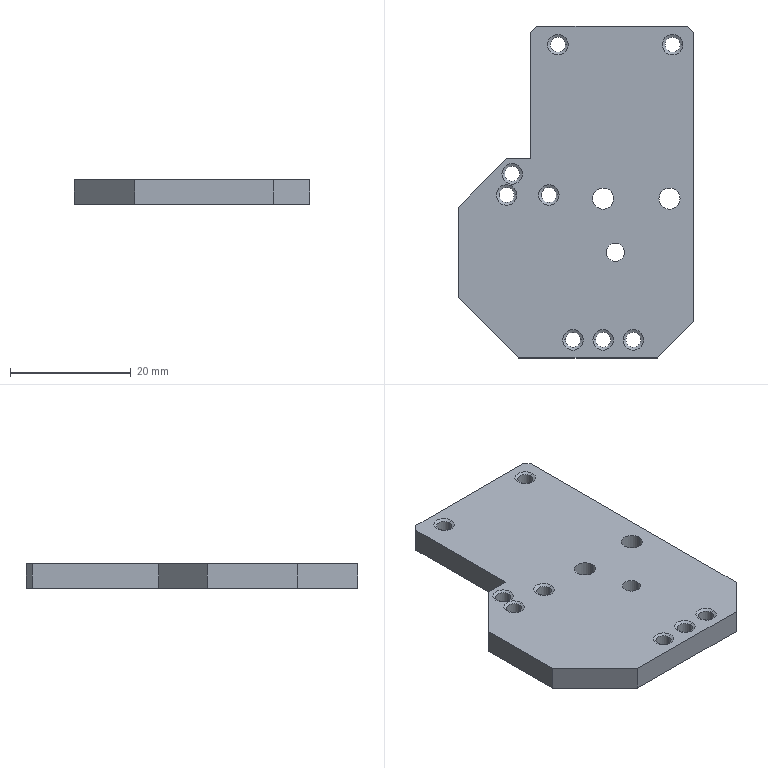Part | NX | 1 solid | 51 faces | box 39 x 55 x 4 mm | volume 6854 mm3 | cylinder 22 | cone 16 | plane 13 | commonest cylinder face diameters 2.5 x16 3.5 x4 3 x2
STEP:
#1=CARTESIAN_POINT('',(-21.5,-2.5,2.));
#2=VERTEX_POINT('',#1);
#3=CARTESIAN_POINT('',(-21.5,-17.5,2.));
#4=VERTEX_POINT('',#3);
#5=CARTESIAN_POINT('',(-21.5,0.,2.));
#6=DIRECTION('',(0.,-1.,0.));
#7=VECTOR('',#6,1000.);
#8=LINE('',#5,#7);
#9=EDGE_CURVE('',#2,#4,#8,.T.);
#10=ORIENTED_EDGE('',*,*,#9,.T.);
#11=CARTESIAN_POINT('',(-11.5,-27.5,2.));
#12=VERTEX_POINT('',#11);
#13=CARTESIAN_POINT('',(-39.,0.,2.));
#14=DIRECTION('',(-0.7071,0.7071,0.));
#15=VECTOR('',#14,1000.);
#16=LINE('',#13,#15);
#17=EDGE_CURVE('',#12,#4,#16,.T.);
#18=ORIENTED_EDGE('',*,*,#17,.F.);
#19=CARTESIAN_POINT('',(11.5,-27.5,2.));
#20=VERTEX_POINT('',#19);
#21=CARTESIAN_POINT('',(0.,-27.5,2.));
#22=DIRECTION('',(-1.,0.,0.));
#23=VECTOR('',#22,1000.);
#24=LINE('',#21,#23);
#25=EDGE_CURVE('',#20,#12,#24,.T.);
#26=ORIENTED_EDGE('',*,*,#25,.F.);
#27=CARTESIAN_POINT('',(17.5,-21.5,2.));
#28=VERTEX_POINT('',#27);
#29=CARTESIAN_POINT('',(39.,0.,2.));
#30=DIRECTION('',(-0.7071,-0.7071,0.));
#31=VECTOR('',#30,1000.);
#32=LINE('',#29,#31);
#33=EDGE_CURVE('',#28,#20,#32,.T.);
#34=ORIENTED_EDGE('',*,*,#33,.F.);
#35=CARTESIAN_POINT('',(17.5,26.5,2.));
#36=VERTEX_POINT('',#35);
#37=CARTESIAN_POINT('',(17.5,0.,2.));
#38=DIRECTION('',(0.,-1.,0.));
#39=VECTOR('',#38,1000.);
#40=LINE('',#37,#39);
#41=EDGE_CURVE('',#36,#28,#40,.T.);
#42=ORIENTED_EDGE('',*,*,#41,.F.);
#43=CARTESIAN_POINT('',(16.5,27.5,2.));
#44=VERTEX_POINT('',#43);
#45=CARTESIAN_POINT('',(44.,0.,2.));
#46=DIRECTION('',(0.7071,-0.7071,0.));
#47=VECTOR('',#46,1000.);
#48=LINE('',#45,#47);
#49=EDGE_CURVE('',#44,#36,#48,.T.);
#50=ORIENTED_EDGE('',*,*,#49,.F.);
#51=CARTESIAN_POINT('',(-8.5,27.5,2.));
#52=VERTEX_POINT('',#51);
#53=CARTESIAN_POINT('',(0.,27.5,2.));
#54=DIRECTION('',(1.,0.,0.));
#55=VECTOR('',#54,1000.);
#56=LINE('',#53,#55);
#57=EDGE_CURVE('',#52,#44,#56,.T.);
#58=ORIENTED_EDGE('',*,*,#57,.F.);
#59=CARTESIAN_POINT('',(-9.5,26.5,2.));
#60=VERTEX_POINT('',#59);
#61=CARTESIAN_POINT('',(-36.,0.,2.));
#62=DIRECTION('',(-0.7071,-0.7071,0.));
#63=VECTOR('',#62,1000.);
#64=LINE('',#61,#63);
#65=EDGE_CURVE('',#52,#60,#64,.T.);
#66=ORIENTED_EDGE('',*,*,#65,.T.);
#67=CARTESIAN_POINT('',(-9.5,5.5,2.));
#68=VERTEX_POINT('',#67);
#69=CARTESIAN_POINT('',(-9.5,0.,2.));
#70=DIRECTION('',(0.,-1.,0.));
#71=VECTOR('',#70,1000.);
#72=LINE('',#69,#71);
#73=EDGE_CURVE('',#60,#68,#72,.T.);
#74=ORIENTED_EDGE('',*,*,#73,.T.);
#75=CARTESIAN_POINT('',(-13.5,5.5,2.));
#76=VERTEX_POINT('',#75);
#77=CARTESIAN_POINT('',(0.,5.5,2.));
#78=DIRECTION('',(-1.,0.,0.));
#79=VECTOR('',#78,1000.);
#80=LINE('',#77,#79);
#81=EDGE_CURVE('',#68,#76,#80,.T.);
#82=ORIENTED_EDGE('',*,*,#81,.T.);
#83=CARTESIAN_POINT('',(-19.,0.,2.));
#84=DIRECTION('',(-0.7071,-0.7071,0.));
#85=VECTOR('',#84,1000.);
#86=LINE('',#83,#85);
#87=EDGE_CURVE('',#76,#2,#86,.T.);
#88=ORIENTED_EDGE('',*,*,#87,.T.);
#89=EDGE_LOOP('',(#10,#18,#26,#34,#42,#50,#58,#66,#74,#82,#88));
#90=FACE_BOUND('',#89,.T.);
#91=CARTESIAN_POINT('',(15.25,-1.1,2.));
#92=VERTEX_POINT('',#91);
#93=CARTESIAN_POINT('',(11.75,-1.1,2.));
#94=VERTEX_POINT('',#93);
#95=CARTESIAN_POINT('',(13.5,-1.1,2.));
#96=DIRECTION('',(0.,0.,1.));
#97=DIRECTION('',(1.,0.,0.));
#98=AXIS2_PLACEMENT_3D('',#95,#96,#97);
#99=CIRCLE('',#98,1.75);
#100=EDGE_CURVE('',#92,#94,#99,.T.);
#101=ORIENTED_EDGE('',*,*,#100,.F.);
#102=CARTESIAN_POINT('',(13.5,-1.1,2.));
#103=DIRECTION('',(0.,0.,1.));
#104=DIRECTION('',(1.,0.,0.));
#105=AXIS2_PLACEMENT_3D('',#102,#103,#104);
#106=CIRCLE('',#105,1.75);
#107=EDGE_CURVE('',#94,#92,#106,.T.);
#108=ORIENTED_EDGE('',*,*,#107,.F.);
#109=EDGE_LOOP('',(#101,#108));
#110=FACE_BOUND('',#109,.T.);
#111=CARTESIAN_POINT('',(0.8,-24.5,2.));
#112=VERTEX_POINT('',#111);
#113=CARTESIAN_POINT('',(4.2,-24.5,2.));
#114=VERTEX_POINT('',#113);
#115=CARTESIAN_POINT('',(2.5,-24.5,2.));
#116=DIRECTION('',(0.,0.,1.));
#117=DIRECTION('',(1.,0.,0.));
#118=AXIS2_PLACEMENT_3D('',#115,#116,#117);
#119=CIRCLE('',#118,1.7);
#120=EDGE_CURVE('',#112,#114,#119,.T.);
#121=ORIENTED_EDGE('',*,*,#120,.F.);
#122=CARTESIAN_POINT('',(2.5,-24.5,2.));
#123=DIRECTION('',(0.,0.,1.));
#124=DIRECTION('',(1.,0.,0.));
#125=AXIS2_PLACEMENT_3D('',#122,#123,#124);
#126=CIRCLE('',#125,1.7);
#127=EDGE_CURVE('',#114,#112,#126,.T.);
#128=ORIENTED_EDGE('',*,*,#127,.F.);
#129=EDGE_LOOP('',(#121,#128));
#130=FACE_BOUND('',#129,.T.);
#131=CARTESIAN_POINT('',(-15.2,-0.5,2.));
#132=VERTEX_POINT('',#131);
#133=CARTESIAN_POINT('',(-11.8,-0.5,2.));
#134=VERTEX_POINT('',#133);
#135=CARTESIAN_POINT('',(-13.5,-0.5,2.));
#136=DIRECTION('',(0.,0.,1.));
#137=DIRECTION('',(1.,0.,0.));
#138=AXIS2_PLACEMENT_3D('',#135,#136,#137);
#139=CIRCLE('',#138,1.7);
#140=EDGE_CURVE('',#132,#134,#139,.T.);
#141=ORIENTED_EDGE('',*,*,#140,.F.);
#142=CARTESIAN_POINT('',(-13.5,-0.5,2.));
#143=DIRECTION('',(0.,0.,1.));
#144=DIRECTION('',(1.,0.,0.));
#145=AXIS2_PLACEMENT_3D('',#142,#143,#144);
#146=CIRCLE('',#145,1.7);
#147=EDGE_CURVE('',#134,#132,#146,.T.);
#148=ORIENTED_EDGE('',*,*,#147,.F.);
#149=EDGE_LOOP('',(#141,#148));
#150=FACE_BOUND('',#149,.T.);
#151=CARTESIAN_POINT('',(4.25,-1.1,2.));
#152=VERTEX_POINT('',#151);
#153=CARTESIAN_POINT('',(0.75,-1.1,2.));
#154=VERTEX_POINT('',#153);
#155=CARTESIAN_POINT('',(2.5,-1.1,2.));
#156=DIRECTION('',(0.,0.,1.));
#157=DIRECTION('',(1.,0.,0.));
#158=AXIS2_PLACEMENT_3D('',#155,#156,#157);
#159=CIRCLE('',#158,1.75);
#160=EDGE_CURVE('',#152,#154,#159,.T.);
#161=ORIENTED_EDGE('',*,*,#160,.F.);
#162=CARTESIAN_POINT('',(2.5,-1.1,2.));
#163=DIRECTION('',(0.,0.,1.));
#164=DIRECTION('',(1.,0.,0.));
#165=AXIS2_PLACEMENT_3D('',#162,#163,#164);
#166=CIRCLE('',#165,1.75);
#167=EDGE_CURVE('',#154,#152,#166,.T.);
#168=ORIENTED_EDGE('',*,*,#167,.F.);
#169=EDGE_LOOP('',(#161,#168));
#170=FACE_BOUND('',#169,.T.);
#171=CARTESIAN_POINT('',(12.3,24.4,2.));
#172=VERTEX_POINT('',#171);
#173=CARTESIAN_POINT('',(15.7,24.4,2.));
#174=VERTEX_POINT('',#173);
#175=CARTESIAN_POINT('',(14.,24.4,2.));
#176=DIRECTION('',(0.,0.,1.));
#177=DIRECTION('',(1.,0.,0.));
#178=AXIS2_PLACEMENT_3D('',#175,#176,#177);
#179=CIRCLE('',#178,1.7);
#180=EDGE_CURVE('',#172,#174,#179,.T.);
#181=ORIENTED_EDGE('',*,*,#180,.F.);
#182=CARTESIAN_POINT('',(14.,24.4,2.));
#183=DIRECTION('',(0.,0.,1.));
#184=DIRECTION('',(1.,0.,0.));
#185=AXIS2_PLACEMENT_3D('',#182,#183,#184);
#186=CIRCLE('',#185,1.7);
#187=EDGE_CURVE('',#174,#172,#186,.T.);
#188=ORIENTED_EDGE('',*,*,#187,.F.);
#189=EDGE_LOOP('',(#181,#188));
#190=FACE_BOUND('',#189,.T.);
#191=CARTESIAN_POINT('',(3.,-10.,2.));
#192=VERTEX_POINT('',#191);
#193=CARTESIAN_POINT('',(6.,-10.,2.));
#194=VERTEX_POINT('',#193);
#195=CARTESIAN_POINT('',(4.5,-10.,2.));
#196=DIRECTION('',(0.,0.,1.));
#197=DIRECTION('',(1.,0.,0.));
#198=AXIS2_PLACEMENT_3D('',#195,#196,#197);
#199=CIRCLE('',#198,1.5);
#200=EDGE_CURVE('',#192,#194,#199,.T.);
#201=ORIENTED_EDGE('',*,*,#200,.F.);
#202=CARTESIAN_POINT('',(4.5,-10.,2.));
#203=DIRECTION('',(0.,0.,1.));
#204=DIRECTION('',(1.,0.,0.));
#205=AXIS2_PLACEMENT_3D('',#202,#203,#204);
#206=CIRCLE('',#205,1.5);
#207=EDGE_CURVE('',#194,#192,#206,.T.);
#208=ORIENTED_EDGE('',*,*,#207,.F.);
#209=EDGE_LOOP('',(#201,#208));
#210=FACE_BOUND('',#209,.T.);
#211=CARTESIAN_POINT('',(-8.2,-0.5,2.));
#212=VERTEX_POINT('',#211);
#213=CARTESIAN_POINT('',(-4.8,-0.5,2.));
#214=VERTEX_POINT('',#213);
#215=CARTESIAN_POINT('',(-6.5,-0.5,2.));
#216=DIRECTION('',(0.,0.,1.));
#217=DIRECTION('',(1.,0.,0.));
#218=AXIS2_PLACEMENT_3D('',#215,#216,#217);
#219=CIRCLE('',#218,1.7);
#220=EDGE_CURVE('',#212,#214,#219,.T.);
#221=ORIENTED_EDGE('',*,*,#220,.F.);
#222=CARTESIAN_POINT('',(-6.5,-0.5,2.));
#223=DIRECTION('',(0.,0.,1.));
#224=DIRECTION('',(1.,0.,0.));
#225=AXIS2_PLACEMENT_3D('',#222,#223,#224);
#226=CIRCLE('',#225,1.7);
#227=EDGE_CURVE('',#214,#212,#226,.T.);
#228=ORIENTED_EDGE('',*,*,#227,.F.);
#229=EDGE_LOOP('',(#221,#228));
#230=FACE_BOUND('',#229,.T.);
#231=CARTESIAN_POINT('',(-3.3,24.4,2.));
#232=VERTEX_POINT('',#231);
#233=CARTESIAN_POINT('',(-6.7,24.4,2.));
#234=VERTEX_POINT('',#233);
#235=CARTESIAN_POINT('',(-5.,24.4,2.));
#236=DIRECTION('',(0.,0.,1.));
#237=DIRECTION('',(1.,0.,0.));
#238=AXIS2_PLACEMENT_3D('',#235,#236,#237);
#239=CIRCLE('',#238,1.7);
#240=EDGE_CURVE('',#232,#234,#239,.T.);
#241=ORIENTED_EDGE('',*,*,#240,.F.);
#242=CARTESIAN_POINT('',(-5.,24.4,2.));
#243=DIRECTION('',(0.,0.,1.));
#244=DIRECTION('',(1.,0.,0.));
#245=AXIS2_PLACEMENT_3D('',#242,#243,#244);
#246=CIRCLE('',#245,1.7);
#247=EDGE_CURVE('',#234,#232,#246,.T.);
#248=ORIENTED_EDGE('',*,*,#247,.F.);
#249=EDGE_LOOP('',(#241,#248));
#250=FACE_BOUND('',#249,.T.);
#251=CARTESIAN_POINT('',(9.2,-24.5,2.));
#252=VERTEX_POINT('',#251);
#253=CARTESIAN_POINT('',(5.8,-24.5,2.));
#254=VERTEX_POINT('',#253);
#255=CARTESIAN_POINT('',(7.5,-24.5,2.));
#256=DIRECTION('',(0.,0.,1.));
#257=DIRECTION('',(1.,0.,0.));
#258=AXIS2_PLACEMENT_3D('',#255,#256,#257);
#259=CIRCLE('',#258,1.7);
#260=EDGE_CURVE('',#252,#254,#259,.T.);
#261=ORIENTED_EDGE('',*,*,#260,.F.);
#262=CARTESIAN_POINT('',(7.5,-24.5,2.));
#263=DIRECTION('',(0.,0.,1.));
#264=DIRECTION('',(1.,0.,0.));
#265=AXIS2_PLACEMENT_3D('',#262,#263,#264);
#266=CIRCLE('',#265,1.7);
#267=EDGE_CURVE('',#254,#252,#266,.T.);
#268=ORIENTED_EDGE('',*,*,#267,.F.);
#269=EDGE_LOOP('',(#261,#268));
#270=FACE_BOUND('',#269,.T.);
#271=CARTESIAN_POINT('',(-4.2,-24.5,2.));
#272=VERTEX_POINT('',#271);
#273=CARTESIAN_POINT('',(-0.8,-24.5,2.));
#274=VERTEX_POINT('',#273);
#275=CARTESIAN_POINT('',(-2.5,-24.5,2.));
#276=DIRECTION('',(0.,0.,1.));
#277=DIRECTION('',(1.,0.,0.));
#278=AXIS2_PLACEMENT_3D('',#275,#276,#277);
#279=CIRCLE('',#278,1.7);
#280=EDGE_CURVE('',#272,#274,#279,.T.);
#281=ORIENTED_EDGE('',*,*,#280,.F.);
#282=CARTESIAN_POINT('',(-2.5,-24.5,2.));
#283=DIRECTION('',(0.,0.,1.));
#284=DIRECTION('',(1.,0.,0.));
#285=AXIS2_PLACEMENT_3D('',#282,#283,#284);
#286=CIRCLE('',#285,1.7);
#287=EDGE_CURVE('',#274,#272,#286,.T.);
#288=ORIENTED_EDGE('',*,*,#287,.F.);
#289=EDGE_LOOP('',(#281,#288));
#290=FACE_BOUND('',#289,.T.);
#291=CARTESIAN_POINT('',(-10.862,3.,2.));
#292=VERTEX_POINT('',#291);
#293=CARTESIAN_POINT('',(-14.262,3.,2.));
#294=VERTEX_POINT('',#293);
#295=CARTESIAN_POINT('',(-12.562,3.,2.));
#296=DIRECTION('',(0.,0.,1.));
#297=DIRECTION('',(1.,0.,0.));
#298=AXIS2_PLACEMENT_3D('',#295,#296,#297);
#299=CIRCLE('',#298,1.7);
#300=EDGE_CURVE('',#292,#294,#299,.T.);
#301=ORIENTED_EDGE('',*,*,#300,.F.);
#302=CARTESIAN_POINT('',(-12.562,3.,2.));
#303=DIRECTION('',(0.,0.,1.));
#304=DIRECTION('',(1.,0.,0.));
#305=AXIS2_PLACEMENT_3D('',#302,#303,#304);
#306=CIRCLE('',#305,1.7);
#307=EDGE_CURVE('',#294,#292,#306,.T.);
#308=ORIENTED_EDGE('',*,*,#307,.F.);
#309=EDGE_LOOP('',(#301,#308));
#310=FACE_BOUND('',#309,.T.);
#311=CARTESIAN_POINT('',(0.,0.,2.));
#312=DIRECTION('',(0.,0.,1.));
#313=DIRECTION('',(1.,0.,0.));
#314=AXIS2_PLACEMENT_3D('',#311,#312,#313);
#315=PLANE('',#314);
#316=ADVANCED_FACE('',(#90,#110,#130,#150,#170,#190,#210,#230,#250,#270,#290,#310),#315,.T.);
#317=CARTESIAN_POINT('',(-21.5,-2.5,-2.));
#318=VERTEX_POINT('',#317);
#319=CARTESIAN_POINT('',(-21.5,-2.5,0.));
#320=DIRECTION('',(0.,0.,1.));
#321=VECTOR('',#320,1000.);
#322=LINE('',#319,#321);
#323=EDGE_CURVE('',#318,#2,#322,.T.);
#324=ORIENTED_EDGE('',*,*,#323,.F.);
#325=CARTESIAN_POINT('',(-21.5,-17.5,-2.));
#326=VERTEX_POINT('',#325);
#327=CARTESIAN_POINT('',(-21.5,0.,-2.));
#328=DIRECTION('',(0.,-1.,0.));
#329=VECTOR('',#328,1000.);
#330=LINE('',#327,#329);
#331=EDGE_CURVE('',#318,#326,#330,.T.);
#332=ORIENTED_EDGE('',*,*,#331,.T.);
#333=CARTESIAN_POINT('',(-21.5,-17.5,0.));
#334=DIRECTION('',(0.,0.,-1.));
#335=VECTOR('',#334,1000.);
#336=LINE('',#333,#335);
#337=EDGE_CURVE('',#4,#326,#336,.T.);
#338=ORIENTED_EDGE('',*,*,#337,.F.);
#339=ORIENTED_EDGE('',*,*,#9,.F.);
#340=EDGE_LOOP('',(#324,#332,#338,#339));
#341=FACE_BOUND('',#340,.T.);
#342=CARTESIAN_POINT('',(-21.5,3.686,-2.));
#343=DIRECTION('',(1.,0.,0.));
#344=DIRECTION('',(0.,1.,0.));
#345=AXIS2_PLACEMENT_3D('',#342,#343,#344);
#346=PLANE('',#345);
#347=ADVANCED_FACE('',(#341),#346,.F.);
#348=CARTESIAN_POINT('',(-1.25,-24.5,1.74));
#349=VERTEX_POINT('',#348);
#350=CARTESIAN_POINT('',(-3.75,-24.5,1.74));
#351=VERTEX_POINT('',#350);
#352=CARTESIAN_POINT('',(-2.5,-24.5,1.74));
#353=DIRECTION('',(0.,0.,1.));
#354=DIRECTION('',(1.,0.,0.));
#355=AXIS2_PLACEMENT_3D('',#352,#353,#354);
#356=CIRCLE('',#355,1.25);
#357=EDGE_CURVE('',#349,#351,#356,.T.);
#358=ORIENTED_EDGE('',*,*,#357,.F.);
#359=CARTESIAN_POINT('',(-1.25,-24.5,1.74));
#360=DIRECTION('',(0.866,0.,0.5));
#361=VECTOR('',#360,1000.);
#362=LINE('',#359,#361);
#363=EDGE_CURVE('',#349,#274,#362,.T.);
#364=ORIENTED_EDGE('',*,*,#363,.T.);
#365=ORIENTED_EDGE('',*,*,#287,.T.);
#366=CARTESIAN_POINT('',(-3.75,-24.5,1.74));
#367=DIRECTION('',(-0.866,0.,0.5));
#368=VECTOR('',#367,1000.);
#369=LINE('',#366,#368);
#370=EDGE_CURVE('',#351,#272,#369,.T.);
#371=ORIENTED_EDGE('',*,*,#370,.F.);
#372=EDGE_LOOP('',(#358,#364,#365,#371));
#373=FACE_BOUND('',#372,.T.);
#374=CARTESIAN_POINT('',(-2.5,-24.5,1.74));
#375=DIRECTION('',(0.,0.,1.));
#376=DIRECTION('',(1.,0.,0.));
#377=AXIS2_PLACEMENT_3D('',#374,#375,#376);
#378=CONICAL_SURFACE('',#377,1.25,1.047);
#379=ADVANCED_FACE('',(#373),#378,.F.);
#380=CARTESIAN_POINT('',(-13.5,5.5,-2.));
#381=VERTEX_POINT('',#380);
#382=CARTESIAN_POINT('',(-13.5,5.5,0.));
#383=DIRECTION('',(0.,0.,-1.));
#384=VECTOR('',#383,1000.);
#385=LINE('',#382,#384);
#386=EDGE_CURVE('',#76,#381,#385,.T.);
#387=ORIENTED_EDGE('',*,*,#386,.F.);
#388=ORIENTED_EDGE('',*,*,#81,.F.);
#389=CARTESIAN_POINT('',(-9.5,5.5,-2.));
#390=VERTEX_POINT('',#389);
#391=CARTESIAN_POINT('',(-9.5,5.5,0.));
#392=DIRECTION('',(0.,0.,-1.));
#393=VECTOR('',#392,1000.);
#394=LINE('',#391,#393);
#395=EDGE_CURVE('',#68,#390,#394,.T.);
#396=ORIENTED_EDGE('',*,*,#395,.T.);
#397=CARTESIAN_POINT('',(0.,5.5,-2.));
#398=DIRECTION('',(-1.,0.,0.));
#399=VECTOR('',#398,1000.);
#400=LINE('',#397,#399);
#401=EDGE_CURVE('',#390,#381,#400,.T.);
#402=ORIENTED_EDGE('',*,*,#401,.T.);
#403=EDGE_LOOP('',(#387,#388,#396,#402));
#404=FACE_BOUND('',#403,.T.);
#405=CARTESIAN_POINT('',(-17.5,5.5,2.));
#406=DIRECTION('',(0.,-1.,0.));
#407=DIRECTION('',(0.,0.,-1.));
#408=AXIS2_PLACEMENT_3D('',#405,#406,#407);
#409=PLANE('',#408);
#410=ADVANCED_FACE('',(#404),#409,.F.);
#411=CARTESIAN_POINT('',(-9.5,26.5,-2.));
#412=VERTEX_POINT('',#411);
#413=CARTESIAN_POINT('',(-9.5,0.,-2.));
#414=DIRECTION('',(0.,-1.,0.));
#415=VECTOR('',#414,1000.);
#416=LINE('',#413,#415);
#417=EDGE_CURVE('',#412,#390,#416,.T.);
#418=ORIENTED_EDGE('',*,*,#417,.T.);
#419=ORIENTED_EDGE('',*,*,#395,.F.);
#420=ORIENTED_EDGE('',*,*,#73,.F.);
#421=CARTESIAN_POINT('',(-9.5,26.5,2.));
#422=DIRECTION('',(0.,0.,-1.));
#423=VECTOR('',#422,1000.);
#424=LINE('',#421,#423);
#425=EDGE_CURVE('',#60,#412,#424,.T.);
#426=ORIENTED_EDGE('',*,*,#425,.T.);
#427=EDGE_LOOP('',(#418,#419,#420,#426));
#428=FACE_BOUND('',#427,.T.);
#429=CARTESIAN_POINT('',(-9.5,5.5,2.));
#430=DIRECTION('',(1.,0.,0.));
#431=DIRECTION('',(0.,1.,0.));
#432=AXIS2_PLACEMENT_3D('',#429,#430,#431);
#433=PLANE('',#432);
#434=ADVANCED_FACE('',(#428),#433,.F.);
#435=CARTESIAN_POINT('',(-8.5,27.5,-2.));
#436=VERTEX_POINT('',#435);
#437=CARTESIAN_POINT('',(-8.5,27.5,2.));
#438=DIRECTION('',(0.,0.,-1.));
#439=VECTOR('',#438,1000.);
#440=LINE('',#437,#439);
#441=EDGE_CURVE('',#52,#436,#440,.T.);
#442=ORIENTED_EDGE('',*,*,#441,.T.);
#443=CARTESIAN_POINT('',(-36.,0.,-2.));
#444=DIRECTION('',(-0.7071,-0.7071,0.));
#445=VECTOR('',#444,1000.);
#446=LINE('',#443,#445);
#447=EDGE_CURVE('',#436,#412,#446,.T.);
#448=ORIENTED_EDGE('',*,*,#447,.T.);
#449=ORIENTED_EDGE('',*,*,#425,.F.);
#450=ORIENTED_EDGE('',*,*,#65,.F.);
#451=EDGE_LOOP('',(#442,#448,#449,#450));
#452=FACE_BOUND('',#451,.T.);
#453=CARTESIAN_POINT('',(-8.5,27.5,-2.));
#454=DIRECTION('',(0.7071,-0.7071,0.));
#455=DIRECTION('',(0.,0.,-1.));
#456=AXIS2_PLACEMENT_3D('',#453,#454,#455);
#457=PLANE('',#456);
#458=ADVANCED_FACE('',(#452),#457,.F.);
#459=ORIENTED_EDGE('',*,*,#441,.F.);
#460=ORIENTED_EDGE('',*,*,#57,.T.);
#461=CARTESIAN_POINT('',(16.5,27.5,-2.));
#462=VERTEX_POINT('',#461);
#463=CARTESIAN_POINT('',(16.5,27.5,2.));
#464=DIRECTION('',(0.,0.,-1.));
#465=VECTOR('',#464,1000.);
#466=LINE('',#463,#465);
#467=EDGE_CURVE('',#44,#462,#466,.T.);
#468=ORIENTED_EDGE('',*,*,#467,.T.);
#469=CARTESIAN_POINT('',(0.,27.5,-2.));
#470=DIRECTION('',(1.,0.,0.));
#471=VECTOR('',#470,1000.);
#472=LINE('',#469,#471);
#473=EDGE_CURVE('',#436,#462,#472,.T.);
#474=ORIENTED_EDGE('',*,*,#473,.F.);
#475=EDGE_LOOP('',(#459,#460,#468,#474));
#476=FACE_BOUND('',#475,.T.);
#477=CARTESIAN_POINT('',(17.5,27.5,-2.));
#478=DIRECTION('',(0.,1.,0.));
#479=DIRECTION('',(1.,0.,0.));
#480=AXIS2_PLACEMENT_3D('',#477,#478,#479);
#481=PLANE('',#480);
#482=ADVANCED_FACE('',(#476),#481,.T.);
#483=ORIENTED_EDGE('',*,*,#467,.F.);
#484=ORIENTED_EDGE('',*,*,#49,.T.);
#485=CARTESIAN_POINT('',(17.5,26.5,-2.));
#486=VERTEX_POINT('',#485);
#487=CARTESIAN_POINT('',(17.5,26.5,2.));
#488=DIRECTION('',(0.,0.,-1.));
#489=VECTOR('',#488,1000.);
#490=LINE('',#487,#489);
#491=EDGE_CURVE('',#36,#486,#490,.T.);
#492=ORIENTED_EDGE('',*,*,#491,.T.);
#493=CARTESIAN_POINT('',(44.,0.,-2.));
#494=DIRECTION('',(0.7071,-0.7071,0.));
#495=VECTOR('',#494,1000.);
#496=LINE('',#493,#495);
#497=EDGE_CURVE('',#462,#486,#496,.T.);
#498=ORIENTED_EDGE('',*,*,#497,.F.);
#499=EDGE_LOOP('',(#483,#484,#492,#498));
#500=FACE_BOUND('',#499,.T.);
#501=CARTESIAN_POINT('',(16.5,27.5,-2.));
#502=DIRECTION('',(0.7071,0.7071,0.));
#503=DIRECTION('',(0.,0.,-1.));
#504=AXIS2_PLACEMENT_3D('',#501,#502,#503);
#505=PLANE('',#504);
#506=ADVANCED_FACE('',(#500),#505,.T.);
#507=CARTESIAN_POINT('',(17.5,-21.5,-2.));
#508=VERTEX_POINT('',#507);
#509=CARTESIAN_POINT('',(17.5,0.,-2.));
#510=DIRECTION('',(0.,-1.,0.));
#511=VECTOR('',#510,1000.);
#512=LINE('',#509,#511);
#513=EDGE_CURVE('',#486,#508,#512,.T.);
#514=ORIENTED_EDGE('',*,*,#513,.F.);
#515=ORIENTED_EDGE('',*,*,#491,.F.);
#516=ORIENTED_EDGE('',*,*,#41,.T.);
#517=CARTESIAN_POINT('',(17.5,-21.5,2.));
#518=DIRECTION('',(0.,0.,-1.));
#519=VECTOR('',#518,1000.);
#520=LINE('',#517,#519);
#521=EDGE_CURVE('',#28,#508,#520,.T.);
#522=ORIENTED_EDGE('',*,*,#521,.T.);
#523=EDGE_LOOP('',(#514,#515,#516,#522));
#524=FACE_BOUND('',#523,.T.);
#525=CARTESIAN_POINT('',(17.5,-27.5,-2.));
#526=DIRECTION('',(1.,0.,0.));
#527=DIRECTION('',(0.,1.,0.));
#528=AXIS2_PLACEMENT_3D('',#525,#526,#527);
#529=PLANE('',#528);
#530=ADVANCED_FACE('',(#524),#529,.T.);
#531=ORIENTED_EDGE('',*,*,#521,.F.);
#532=ORIENTED_EDGE('',*,*,#33,.T.);
#533=CARTESIAN_POINT('',(11.5,-27.5,-2.));
#534=VERTEX_POINT('',#533);
#535=CARTESIAN_POINT('',(11.5,-27.5,2.));
#536=DIRECTION('',(0.,0.,-1.));
#537=VECTOR('',#536,1000.);
#538=LINE('',#535,#537);
#539=EDGE_CURVE('',#20,#534,#538,.T.);
#540=ORIENTED_EDGE('',*,*,#539,.T.);
#541=CARTESIAN_POINT('',(39.,0.,-2.));
#542=DIRECTION('',(-0.7071,-0.7071,0.));
#543=VECTOR('',#542,1000.);
#544=LINE('',#541,#543);
#545=EDGE_CURVE('',#508,#534,#544,.T.);
#546=ORIENTED_EDGE('',*,*,#545,.F.);
#547=EDGE_LOOP('',(#531,#532,#540,#546));
#548=FACE_BOUND('',#547,.T.);
#549=CARTESIAN_POINT('',(17.5,-21.5,-2.));
#550=DIRECTION('',(0.7071,-0.7071,0.));
#551=DIRECTION('',(0.,0.,-1.));
#552=AXIS2_PLACEMENT_3D('',#549,#550,#551);
#553=PLANE('',#552);
#554=ADVANCED_FACE('',(#548),#553,.T.);
#555=CARTESIAN_POINT('',(-11.5,-27.5,-2.));
#556=VERTEX_POINT('',#555);
#557=CARTESIAN_POINT('',(0.,-27.5,-2.));
#558=DIRECTION('',(-1.,0.,0.));
#559=VECTOR('',#558,1000.);
#560=LINE('',#557,#559);
#561=EDGE_CURVE('',#534,#556,#560,.T.);
#562=ORIENTED_EDGE('',*,*,#561,.F.);
#563=ORIENTED_EDGE('',*,*,#539,.F.);
#564=ORIENTED_EDGE('',*,*,#25,.T.);
#565=CARTESIAN_POINT('',(-11.5,-27.5,0.));
#566=DIRECTION('',(0.,0.,-1.));
#567=VECTOR('',#566,1000.);
#568=LINE('',#565,#567);
#569=EDGE_CURVE('',#12,#556,#568,.T.);
#570=ORIENTED_EDGE('',*,*,#569,.T.);
#571=EDGE_LOOP('',(#562,#563,#564,#570));
#572=FACE_BOUND('',#571,.T.);
#573=CARTESIAN_POINT('',(-17.5,-27.5,-2.));
#574=DIRECTION('',(0.,-1.,0.));
#575=DIRECTION('',(0.,0.,-1.));
#576=AXIS2_PLACEMENT_3D('',#573,#574,#575);
#577=PLANE('',#576);
#578=ADVANCED_FACE('',(#572),#577,.T.);
#579=ORIENTED_EDGE('',*,*,#337,.T.);
#580=CARTESIAN_POINT('',(-39.,0.,-2.));
#581=DIRECTION('',(-0.7071,0.7071,0.));
#582=VECTOR('',#581,1000.);
#583=LINE('',#580,#582);
#584=EDGE_CURVE('',#556,#326,#583,.T.);
#585=ORIENTED_EDGE('',*,*,#584,.F.);
#586=ORIENTED_EDGE('',*,*,#569,.F.);
#587=ORIENTED_EDGE('',*,*,#17,.T.);
#588=EDGE_LOOP('',(#579,#585,#586,#587));
#589=FACE_BOUND('',#588,.T.);
#590=CARTESIAN_POINT('',(-11.5,-27.5,-2.));
#591=DIRECTION('',(-0.7071,-0.7071,0.));
#592=DIRECTION('',(-0.7071,0.7071,0.));
#593=AXIS2_PLACEMENT_3D('',#590,#591,#592);
#594=PLANE('',#593);
#595=ADVANCED_FACE('',(#589),#594,.T.);
#596=ORIENTED_EDGE('',*,*,#401,.F.);
#597=ORIENTED_EDGE('',*,*,#417,.F.);
#598=ORIENTED_EDGE('',*,*,#447,.F.);
#599=ORIENTED_EDGE('',*,*,#473,.T.);
#600=ORIENTED_EDGE('',*,*,#497,.T.);
#601=ORIENTED_EDGE('',*,*,#513,.T.);
#602=ORIENTED_EDGE('',*,*,#545,.T.);
#603=ORIENTED_EDGE('',*,*,#561,.T.);
#604=ORIENTED_EDGE('',*,*,#584,.T.);
#605=ORIENTED_EDGE('',*,*,#331,.F.);
#606=CARTESIAN_POINT('',(-19.,0.,-2.));
#607=DIRECTION('',(-0.7071,-0.7071,0.));
#608=VECTOR('',#607,1000.);
#609=LINE('',#606,#608);
#610=EDGE_CURVE('',#381,#318,#609,.T.);
#611=ORIENTED_EDGE('',*,*,#610,.F.);
#612=EDGE_LOOP('',(#596,#597,#598,#599,#600,#601,#602,#603,#604,#605,#611));
#613=FACE_BOUND('',#612,.T.);
#614=CARTESIAN_POINT('',(15.25,-1.1,-2.));
#615=VERTEX_POINT('',#614);
#616=CARTESIAN_POINT('',(11.75,-1.1,-2.));
#617=VERTEX_POINT('',#616);
#618=CARTESIAN_POINT('',(13.5,-1.1,-2.));
#619=DIRECTION('',(0.,0.,1.));
#620=DIRECTION('',(1.,0.,0.));
#621=AXIS2_PLACEMENT_3D('',#618,#619,#620);
#622=CIRCLE('',#621,1.75);
#623=EDGE_CURVE('',#615,#617,#622,.T.);
#624=ORIENTED_EDGE('',*,*,#623,.T.);
#625=CARTESIAN_POINT('',(13.5,-1.1,-2.));
#626=DIRECTION('',(0.,0.,1.));
#627=DIRECTION('',(1.,0.,0.));
#628=AXIS2_PLACEMENT_3D('',#625,#626,#627);
#629=CIRCLE('',#628,1.75);
#630=EDGE_CURVE('',#617,#615,#629,.T.);
#631=ORIENTED_EDGE('',*,*,#630,.T.);
#632=EDGE_LOOP('',(#624,#631));
#633=FACE_BOUND('',#632,.T.);
#634=CARTESIAN_POINT('',(-11.312,3.,-2.));
#635=VERTEX_POINT('',#634);
#636=CARTESIAN_POINT('',(-13.812,3.,-2.));
#637=VERTEX_POINT('',#636);
#638=CARTESIAN_POINT('',(-12.562,3.,-2.));
#639=DIRECTION('',(0.,0.,1.));
#640=DIRECTION('',(1.,0.,0.));
#641=AXIS2_PLACEMENT_3D('',#638,#639,#640);
#642=CIRCLE('',#641,1.25);
#643=EDGE_CURVE('',#635,#637,#642,.T.);
#644=ORIENTED_EDGE('',*,*,#643,.T.);
#645=CARTESIAN_POINT('',(-12.562,3.,-2.));
#646=DIRECTION('',(0.,0.,1.));
#647=DIRECTION('',(1.,0.,0.));
#648=AXIS2_PLACEMENT_3D('',#645,#646,#647);
#649=CIRCLE('',#648,1.25);
#650=EDGE_CURVE('',#637,#635,#649,.T.);
#651=ORIENTED_EDGE('',*,*,#650,.T.);
#652=EDGE_LOOP('',(#644,#651));
#653=FACE_BOUND('',#652,.T.);
#654=CARTESIAN_POINT('',(3.,-10.,-2.));
#655=VERTEX_POINT('',#654);
#656=CARTESIAN_POINT('',(6.,-10.,-2.));
#657=VERTEX_POINT('',#656);
#658=CARTESIAN_POINT('',(4.5,-10.,-2.));
#659=DIRECTION('',(0.,0.,1.));
#660=DIRECTION('',(1.,0.,0.));
#661=AXIS2_PLACEMENT_3D('',#658,#659,#660);
#662=CIRCLE('',#661,1.5);
#663=EDGE_CURVE('',#655,#657,#662,.T.);
#664=ORIENTED_EDGE('',*,*,#663,.T.);
#665=CARTESIAN_POINT('',(4.5,-10.,-2.));
#666=DIRECTION('',(0.,0.,1.));
#667=DIRECTION('',(1.,0.,0.));
#668=AXIS2_PLACEMENT_3D('',#665,#666,#667);
#669=CIRCLE('',#668,1.5);
#670=EDGE_CURVE('',#657,#655,#669,.T.);
#671=ORIENTED_EDGE('',*,*,#670,.T.);
#672=EDGE_LOOP('',(#664,#671));
#673=FACE_BOUND('',#672,.T.);
#674=CARTESIAN_POINT('',(-14.75,-0.5,-2.));
#675=VERTEX_POINT('',#674);
#676=CARTESIAN_POINT('',(-12.25,-0.5,-2.));
#677=VERTEX_POINT('',#676);
#678=CARTESIAN_POINT('',(-13.5,-0.5,-2.));
#679=DIRECTION('',(0.,0.,1.));
#680=DIRECTION('',(1.,0.,0.));
#681=AXIS2_PLACEMENT_3D('',#678,#679,#680);
#682=CIRCLE('',#681,1.25);
#683=EDGE_CURVE('',#675,#677,#682,.T.);
#684=ORIENTED_EDGE('',*,*,#683,.T.);
#685=CARTESIAN_POINT('',(-13.5,-0.5,-2.));
#686=DIRECTION('',(0.,0.,1.));
#687=DIRECTION('',(1.,0.,0.));
#688=AXIS2_PLACEMENT_3D('',#685,#686,#687);
#689=CIRCLE('',#688,1.25);
#690=EDGE_CURVE('',#677,#675,#689,.T.);
#691=ORIENTED_EDGE('',*,*,#690,.T.);
#692=EDGE_LOOP('',(#684,#691));
#693=FACE_BOUND('',#692,.T.);
#694=CARTESIAN_POINT('',(-5.25,-0.5,-2.));
#695=VERTEX_POINT('',#694);
#696=CARTESIAN_POINT('',(-7.75,-0.5,-2.));
#697=VERTEX_POINT('',#696);
#698=CARTESIAN_POINT('',(-6.5,-0.5,-2.));
#699=DIRECTION('',(0.,0.,1.));
#700=DIRECTION('',(1.,0.,0.));
#701=AXIS2_PLACEMENT_3D('',#698,#699,#700);
#702=CIRCLE('',#701,1.25);
#703=EDGE_CURVE('',#695,#697,#702,.T.);
#704=ORIENTED_EDGE('',*,*,#703,.T.);
#705=CARTESIAN_POINT('',(-6.5,-0.5,-2.));
#706=DIRECTION('',(0.,0.,1.));
#707=DIRECTION('',(1.,0.,0.));
#708=AXIS2_PLACEMENT_3D('',#705,#706,#707);
#709=CIRCLE('',#708,1.25);
#710=EDGE_CURVE('',#697,#695,#709,.T.);
#711=ORIENTED_EDGE('',*,*,#710,.T.);
#712=EDGE_LOOP('',(#704,#711));
#713=FACE_BOUND('',#712,.T.);
#714=CARTESIAN_POINT('',(4.25,-1.1,-2.));
#715=VERTEX_POINT('',#714);
#716=CARTESIAN_POINT('',(0.75,-1.1,-2.));
#717=VERTEX_POINT('',#716);
#718=CARTESIAN_POINT('',(2.5,-1.1,-2.));
#719=DIRECTION('',(0.,0.,1.));
#720=DIRECTION('',(1.,0.,0.));
#721=AXIS2_PLACEMENT_3D('',#718,#719,#720);
#722=CIRCLE('',#721,1.75);
#723=EDGE_CURVE('',#715,#717,#722,.T.);
#724=ORIENTED_EDGE('',*,*,#723,.T.);
#725=CARTESIAN_POINT('',(2.5,-1.1,-2.));
#726=DIRECTION('',(0.,0.,1.));
#727=DIRECTION('',(1.,0.,0.));
#728=AXIS2_PLACEMENT_3D('',#725,#726,#727);
#729=CIRCLE('',#728,1.75);
#730=EDGE_CURVE('',#717,#715,#729,.T.);
#731=ORIENTED_EDGE('',*,*,#730,.T.);
#732=EDGE_LOOP('',(#724,#731));
#733=FACE_BOUND('',#732,.T.);
#734=CARTESIAN_POINT('',(-3.75,24.4,-2.));
#735=VERTEX_POINT('',#734);
#736=CARTESIAN_POINT('',(-6.25,24.4,-2.));
#737=VERTEX_POINT('',#736);
#738=CARTESIAN_POINT('',(-5.,24.4,-2.));
#739=DIRECTION('',(0.,0.,1.));
#740=DIRECTION('',(1.,0.,0.));
#741=AXIS2_PLACEMENT_3D('',#738,#739,#740);
#742=CIRCLE('',#741,1.25);
#743=EDGE_CURVE('',#735,#737,#742,.T.);
#744=ORIENTED_EDGE('',*,*,#743,.T.);
#745=CARTESIAN_POINT('',(-5.,24.4,-2.));
#746=DIRECTION('',(0.,0.,1.));
#747=DIRECTION('',(1.,0.,0.));
#748=AXIS2_PLACEMENT_3D('',#745,#746,#747);
#749=CIRCLE('',#748,1.25);
#750=EDGE_CURVE('',#737,#735,#749,.T.);
#751=ORIENTED_EDGE('',*,*,#750,.T.);
#752=EDGE_LOOP('',(#744,#751));
#753=FACE_BOUND('',#752,.T.);
#754=CARTESIAN_POINT('',(15.25,24.4,-2.));
#755=VERTEX_POINT('',#754);
#756=CARTESIAN_POINT('',(12.75,24.4,-2.));
#757=VERTEX_POINT('',#756);
#758=CARTESIAN_POINT('',(14.,24.4,-2.));
#759=DIRECTION('',(0.,0.,1.));
#760=DIRECTION('',(1.,0.,0.));
#761=AXIS2_PLACEMENT_3D('',#758,#759,#760);
#762=CIRCLE('',#761,1.25);
#763=EDGE_CURVE('',#755,#757,#762,.T.);
#764=ORIENTED_EDGE('',*,*,#763,.T.);
#765=CARTESIAN_POINT('',(14.,24.4,-2.));
#766=DIRECTION('',(0.,0.,1.));
#767=DIRECTION('',(1.,0.,0.));
#768=AXIS2_PLACEMENT_3D('',#765,#766,#767);
#769=CIRCLE('',#768,1.25);
#770=EDGE_CURVE('',#757,#755,#769,.T.);
#771=ORIENTED_EDGE('',*,*,#770,.T.);
#772=EDGE_LOOP('',(#764,#771));
#773=FACE_BOUND('',#772,.T.);
#774=CARTESIAN_POINT('',(8.75,-24.5,-2.));
#775=VERTEX_POINT('',#774);
#776=CARTESIAN_POINT('',(6.25,-24.5,-2.));
#777=VERTEX_POINT('',#776);
#778=CARTESIAN_POINT('',(7.5,-24.5,-2.));
#779=DIRECTION('',(0.,0.,1.));
#780=DIRECTION('',(1.,0.,0.));
#781=AXIS2_PLACEMENT_3D('',#778,#779,#780);
#782=CIRCLE('',#781,1.25);
#783=EDGE_CURVE('',#775,#777,#782,.T.);
#784=ORIENTED_EDGE('',*,*,#783,.T.);
#785=CARTESIAN_POINT('',(7.5,-24.5,-2.));
#786=DIRECTION('',(0.,0.,1.));
#787=DIRECTION('',(1.,0.,0.));
#788=AXIS2_PLACEMENT_3D('',#785,#786,#787);
#789=CIRCLE('',#788,1.25);
#790=EDGE_CURVE('',#777,#775,#789,.T.);
#791=ORIENTED_EDGE('',*,*,#790,.T.);
#792=EDGE_LOOP('',(#784,#791));
#793=FACE_BOUND('',#792,.T.);
#794=CARTESIAN_POINT('',(1.25,-24.5,-2.));
#795=VERTEX_POINT('',#794);
#796=CARTESIAN_POINT('',(3.75,-24.5,-2.));
#797=VERTEX_POINT('',#796);
#798=CARTESIAN_POINT('',(2.5,-24.5,-2.));
#799=DIRECTION('',(0.,0.,1.));
#800=DIRECTION('',(1.,0.,0.));
#801=AXIS2_PLACEMENT_3D('',#798,#799,#800);
#802=CIRCLE('',#801,1.25);
#803=EDGE_CURVE('',#795,#797,#802,.T.);
#804=ORIENTED_EDGE('',*,*,#803,.T.);
#805=CARTESIAN_POINT('',(2.5,-24.5,-2.));
#806=DIRECTION('',(0.,0.,1.));
#807=DIRECTION('',(1.,0.,0.));
#808=AXIS2_PLACEMENT_3D('',#805,#806,#807);
#809=CIRCLE('',#808,1.25);
#810=EDGE_CURVE('',#797,#795,#809,.T.);
#811=ORIENTED_EDGE('',*,*,#810,.T.);
#812=EDGE_LOOP('',(#804,#811));
#813=FACE_BOUND('',#812,.T.);
#814=CARTESIAN_POINT('',(-1.25,-24.5,-2.));
#815=VERTEX_POINT('',#814);
#816=CARTESIAN_POINT('',(-3.75,-24.5,-2.));
#817=VERTEX_POINT('',#816);
#818=CARTESIAN_POINT('',(-2.5,-24.5,-2.));
#819=DIRECTION('',(0.,0.,1.));
#820=DIRECTION('',(1.,0.,0.));
#821=AXIS2_PLACEMENT_3D('',#818,#819,#820);
#822=CIRCLE('',#821,1.25);
#823=EDGE_CURVE('',#815,#817,#822,.T.);
#824=ORIENTED_EDGE('',*,*,#823,.T.);
#825=CARTESIAN_POINT('',(-2.5,-24.5,-2.));
#826=DIRECTION('',(0.,0.,1.));
#827=DIRECTION('',(1.,0.,0.));
#828=AXIS2_PLACEMENT_3D('',#825,#826,#827);
#829=CIRCLE('',#828,1.25);
#830=EDGE_CURVE('',#817,#815,#829,.T.);
#831=ORIENTED_EDGE('',*,*,#830,.T.);
#832=EDGE_LOOP('',(#824,#831));
#833=FACE_BOUND('',#832,.T.);
#834=CARTESIAN_POINT('',(0.,0.,-2.));
#835=DIRECTION('',(0.,0.,1.));
#836=DIRECTION('',(1.,0.,0.));
#837=AXIS2_PLACEMENT_3D('',#834,#835,#836);
#838=PLANE('',#837);
#839=ADVANCED_FACE('',(#613,#633,#653,#673,#693,#713,#733,#753,#773,#793,#813,#833),#838,.F.);
#840=ORIENTED_EDGE('',*,*,#100,.T.);
#841=CARTESIAN_POINT('',(11.75,-1.1,-2.));
#842=DIRECTION('',(0.,0.,1.));
#843=VECTOR('',#842,1000.);
#844=LINE('',#841,#843);
#845=EDGE_CURVE('',#617,#94,#844,.T.);
#846=ORIENTED_EDGE('',*,*,#845,.F.);
#847=ORIENTED_EDGE('',*,*,#623,.F.);
#848=CARTESIAN_POINT('',(15.25,-1.1,-2.));
#849=DIRECTION('',(0.,0.,1.));
#850=VECTOR('',#849,1000.);
#851=LINE('',#848,#850);
#852=EDGE_CURVE('',#615,#92,#851,.T.);
#853=ORIENTED_EDGE('',*,*,#852,.T.);
#854=EDGE_LOOP('',(#840,#846,#847,#853));
#855=FACE_BOUND('',#854,.T.);
#856=CARTESIAN_POINT('',(13.5,-1.1,-2.));
#857=DIRECTION('',(0.,0.,1.));
#858=DIRECTION('',(1.,0.,0.));
#859=AXIS2_PLACEMENT_3D('',#856,#857,#858);
#860=CYLINDRICAL_SURFACE('',#859,1.75);
#861=ADVANCED_FACE('',(#855),#860,.F.);
#862=ORIENTED_EDGE('',*,*,#180,.T.);
#863=CARTESIAN_POINT('',(15.25,24.4,1.74));
#864=VERTEX_POINT('',#863);
#865=CARTESIAN_POINT('',(15.25,24.4,1.74));
#866=DIRECTION('',(0.866,0.,0.5));
#867=VECTOR('',#866,1000.);
#868=LINE('',#865,#867);
#869=EDGE_CURVE('',#864,#174,#868,.T.);
#870=ORIENTED_EDGE('',*,*,#869,.F.);
#871=CARTESIAN_POINT('',(12.75,24.4,1.74));
#872=VERTEX_POINT('',#871);
#873=CARTESIAN_POINT('',(14.,24.4,1.74));
#874=DIRECTION('',(0.,0.,1.));
#875=DIRECTION('',(1.,0.,0.));
#876=AXIS2_PLACEMENT_3D('',#873,#874,#875);
#877=CIRCLE('',#876,1.25);
#878=EDGE_CURVE('',#872,#864,#877,.T.);
#879=ORIENTED_EDGE('',*,*,#878,.F.);
#880=CARTESIAN_POINT('',(12.75,24.4,1.74));
#881=DIRECTION('',(-0.866,0.,0.5));
#882=VECTOR('',#881,1000.);
#883=LINE('',#880,#882);
#884=EDGE_CURVE('',#872,#172,#883,.T.);
#885=ORIENTED_EDGE('',*,*,#884,.T.);
#886=EDGE_LOOP('',(#862,#870,#879,#885));
#887=FACE_BOUND('',#886,.T.);
#888=CARTESIAN_POINT('',(14.,24.4,1.74));
#889=DIRECTION('',(0.,0.,1.));
#890=DIRECTION('',(1.,0.,0.));
#891=AXIS2_PLACEMENT_3D('',#888,#889,#890);
#892=CONICAL_SURFACE('',#891,1.25,1.047);
#893=ADVANCED_FACE('',(#887),#892,.F.);
#894=ORIENTED_EDGE('',*,*,#200,.T.);
#895=CARTESIAN_POINT('',(6.,-10.,-2.));
#896=DIRECTION('',(0.,0.,1.));
#897=VECTOR('',#896,1000.);
#898=LINE('',#895,#897);
#899=EDGE_CURVE('',#657,#194,#898,.T.);
#900=ORIENTED_EDGE('',*,*,#899,.F.);
#901=ORIENTED_EDGE('',*,*,#663,.F.);
#902=CARTESIAN_POINT('',(3.,-10.,-2.));
#903=DIRECTION('',(0.,0.,1.));
#904=VECTOR('',#903,1000.);
#905=LINE('',#902,#904);
#906=EDGE_CURVE('',#655,#192,#905,.T.);
#907=ORIENTED_EDGE('',*,*,#906,.T.);
#908=EDGE_LOOP('',(#894,#900,#901,#907));
#909=FACE_BOUND('',#908,.T.);
#910=CARTESIAN_POINT('',(4.5,-10.,-2.));
#911=DIRECTION('',(0.,0.,1.));
#912=DIRECTION('',(1.,0.,0.));
#913=AXIS2_PLACEMENT_3D('',#910,#911,#912);
#914=CYLINDRICAL_SURFACE('',#913,1.5);
#915=ADVANCED_FACE('',(#909),#914,.F.);
#916=ORIENTED_EDGE('',*,*,#240,.T.);
#917=CARTESIAN_POINT('',(-6.25,24.4,1.74));
#918=VERTEX_POINT('',#917);
#919=CARTESIAN_POINT('',(-6.25,24.4,1.74));
#920=DIRECTION('',(-0.866,0.,0.5));
#921=VECTOR('',#920,1000.);
#922=LINE('',#919,#921);
#923=EDGE_CURVE('',#234,#918,#922,.F.);
#924=ORIENTED_EDGE('',*,*,#923,.T.);
#925=CARTESIAN_POINT('',(-3.75,24.4,1.74));
#926=VERTEX_POINT('',#925);
#927=CARTESIAN_POINT('',(-5.,24.4,1.74));
#928=DIRECTION('',(0.,0.,1.));
#929=DIRECTION('',(1.,0.,0.));
#930=AXIS2_PLACEMENT_3D('',#927,#928,#929);
#931=CIRCLE('',#930,1.25);
#932=EDGE_CURVE('',#926,#918,#931,.T.);
#933=ORIENTED_EDGE('',*,*,#932,.F.);
#934=CARTESIAN_POINT('',(-3.75,24.4,1.74));
#935=DIRECTION('',(0.866,0.,0.5));
#936=VECTOR('',#935,1000.);
#937=LINE('',#934,#936);
#938=EDGE_CURVE('',#232,#926,#937,.F.);
#939=ORIENTED_EDGE('',*,*,#938,.F.);
#940=EDGE_LOOP('',(#916,#924,#933,#939));
#941=FACE_BOUND('',#940,.T.);
#942=CARTESIAN_POINT('',(-5.,24.4,1.74));
#943=DIRECTION('',(0.,0.,1.));
#944=DIRECTION('',(1.,0.,0.));
#945=AXIS2_PLACEMENT_3D('',#942,#943,#944);
#946=CONICAL_SURFACE('',#945,1.25,1.047);
#947=ADVANCED_FACE('',(#941),#946,.F.);
#948=CARTESIAN_POINT('',(-14.75,-0.5,1.74));
#949=VERTEX_POINT('',#948);
#950=CARTESIAN_POINT('',(-12.25,-0.5,1.74));
#951=VERTEX_POINT('',#950);
#952=CARTESIAN_POINT('',(-13.5,-0.5,1.74));
#953=DIRECTION('',(0.,0.,1.));
#954=DIRECTION('',(1.,0.,0.));
#955=AXIS2_PLACEMENT_3D('',#952,#953,#954);
#956=CIRCLE('',#955,1.25);
#957=EDGE_CURVE('',#949,#951,#956,.T.);
#958=ORIENTED_EDGE('',*,*,#957,.F.);
#959=CARTESIAN_POINT('',(-14.75,-0.5,1.74));
#960=DIRECTION('',(-0.866,0.,0.5));
#961=VECTOR('',#960,1000.);
#962=LINE('',#959,#961);
#963=EDGE_CURVE('',#949,#132,#962,.T.);
#964=ORIENTED_EDGE('',*,*,#963,.T.);
#965=ORIENTED_EDGE('',*,*,#140,.T.);
#966=CARTESIAN_POINT('',(-12.25,-0.5,1.74));
#967=DIRECTION('',(0.866,0.,0.5));
#968=VECTOR('',#967,1000.);
#969=LINE('',#966,#968);
#970=EDGE_CURVE('',#951,#134,#969,.T.);
#971=ORIENTED_EDGE('',*,*,#970,.F.);
#972=EDGE_LOOP('',(#958,#964,#965,#971));
#973=FACE_BOUND('',#972,.T.);
#974=CARTESIAN_POINT('',(-13.5,-0.5,1.74));
#975=DIRECTION('',(0.,0.,1.));
#976=DIRECTION('',(1.,0.,0.));
#977=AXIS2_PLACEMENT_3D('',#974,#975,#976);
#978=CONICAL_SURFACE('',#977,1.25,1.047);
#979=ADVANCED_FACE('',(#973),#978,.F.);
#980=CARTESIAN_POINT('',(-5.,24.4,1.74));
#981=DIRECTION('',(0.,0.,1.));
#982=DIRECTION('',(1.,0.,0.));
#983=AXIS2_PLACEMENT_3D('',#980,#981,#982);
#984=CIRCLE('',#983,1.25);
#985=EDGE_CURVE('',#918,#926,#984,.T.);
#986=ORIENTED_EDGE('',*,*,#985,.T.);
#987=CARTESIAN_POINT('',(-3.75,24.4,2.));
#988=DIRECTION('',(0.,0.,1.));
#989=VECTOR('',#988,1000.);
#990=LINE('',#987,#989);
#991=EDGE_CURVE('',#735,#926,#990,.T.);
#992=ORIENTED_EDGE('',*,*,#991,.F.);
#993=ORIENTED_EDGE('',*,*,#750,.F.);
#994=CARTESIAN_POINT('',(-6.25,24.4,2.));
#995=DIRECTION('',(0.,0.,1.));
#996=VECTOR('',#995,1000.);
#997=LINE('',#994,#996);
#998=EDGE_CURVE('',#737,#918,#997,.T.);
#999=ORIENTED_EDGE('',*,*,#998,.T.);
#1000=EDGE_LOOP('',(#986,#992,#993,#999));
#1001=FACE_BOUND('',#1000,.T.);
#1002=CARTESIAN_POINT('',(-5.,24.4,2.));
#1003=DIRECTION('',(0.,0.,1.));
#1004=DIRECTION('',(1.,0.,0.));
#1005=AXIS2_PLACEMENT_3D('',#1002,#1003,#1004);
#1006=CYLINDRICAL_SURFACE('',#1005,1.25);
#1007=ADVANCED_FACE('',(#1001),#1006,.F.);
#1008=ORIENTED_EDGE('',*,*,#957,.T.);
#1009=CARTESIAN_POINT('',(-12.25,-0.5,2.));
#1010=DIRECTION('',(0.,0.,1.));
#1011=VECTOR('',#1010,1000.);
#1012=LINE('',#1009,#1011);
#1013=EDGE_CURVE('',#677,#951,#1012,.T.);
#1014=ORIENTED_EDGE('',*,*,#1013,.F.);
#1015=ORIENTED_EDGE('',*,*,#683,.F.);
#1016=CARTESIAN_POINT('',(-14.75,-0.5,2.));
#1017=DIRECTION('',(0.,0.,1.));
#1018=VECTOR('',#1017,1000.);
#1019=LINE('',#1016,#1018);
#1020=EDGE_CURVE('',#675,#949,#1019,.T.);
#1021=ORIENTED_EDGE('',*,*,#1020,.T.);
#1022=EDGE_LOOP('',(#1008,#1014,#1015,#1021));
#1023=FACE_BOUND('',#1022,.T.);
#1024=CARTESIAN_POINT('',(-13.5,-0.5,2.));
#1025=DIRECTION('',(0.,0.,1.));
#1026=DIRECTION('',(1.,0.,0.));
#1027=AXIS2_PLACEMENT_3D('',#1024,#1025,#1026);
#1028=CYLINDRICAL_SURFACE('',#1027,1.25);
#1029=ADVANCED_FACE('',(#1023),#1028,.F.);
#1030=ORIENTED_EDGE('',*,*,#723,.F.);
#1031=CARTESIAN_POINT('',(4.25,-1.1,-2.));
#1032=DIRECTION('',(0.,0.,1.));
#1033=VECTOR('',#1032,1000.);
#1034=LINE('',#1031,#1033);
#1035=EDGE_CURVE('',#715,#152,#1034,.T.);
#1036=ORIENTED_EDGE('',*,*,#1035,.T.);
#1037=ORIENTED_EDGE('',*,*,#160,.T.);
#1038=CARTESIAN_POINT('',(0.75,-1.1,-2.));
#1039=DIRECTION('',(0.,0.,1.));
#1040=VECTOR('',#1039,1000.);
#1041=LINE('',#1038,#1040);
#1042=EDGE_CURVE('',#717,#154,#1041,.T.);
#1043=ORIENTED_EDGE('',*,*,#1042,.F.);
#1044=EDGE_LOOP('',(#1030,#1036,#1037,#1043));
#1045=FACE_BOUND('',#1044,.T.);
#1046=CARTESIAN_POINT('',(2.5,-1.1,-2.));
#1047=DIRECTION('',(0.,0.,1.));
#1048=DIRECTION('',(1.,0.,0.));
#1049=AXIS2_PLACEMENT_3D('',#1046,#1047,#1048);
#1050=CYLINDRICAL_SURFACE('',#1049,1.75);
#1051=ADVANCED_FACE('',(#1045),#1050,.F.);
#1052=ORIENTED_EDGE('',*,*,#703,.F.);
#1053=CARTESIAN_POINT('',(-5.25,-0.5,1.74));
#1054=VERTEX_POINT('',#1053);
#1055=CARTESIAN_POINT('',(-5.25,-0.5,2.));
#1056=DIRECTION('',(0.,0.,1.));
#1057=VECTOR('',#1056,1000.);
#1058=LINE('',#1055,#1057);
#1059=EDGE_CURVE('',#695,#1054,#1058,.T.);
#1060=ORIENTED_EDGE('',*,*,#1059,.T.);
#1061=CARTESIAN_POINT('',(-7.75,-0.5,1.74));
#1062=VERTEX_POINT('',#1061);
#1063=CARTESIAN_POINT('',(-6.5,-0.5,1.74));
#1064=DIRECTION('',(0.,0.,1.));
#1065=DIRECTION('',(1.,0.,0.));
#1066=AXIS2_PLACEMENT_3D('',#1063,#1064,#1065);
#1067=CIRCLE('',#1066,1.25);
#1068=EDGE_CURVE('',#1054,#1062,#1067,.T.);
#1069=ORIENTED_EDGE('',*,*,#1068,.T.);
#1070=CARTESIAN_POINT('',(-7.75,-0.5,2.));
#1071=DIRECTION('',(0.,0.,1.));
#1072=VECTOR('',#1071,1000.);
#1073=LINE('',#1070,#1072);
#1074=EDGE_CURVE('',#697,#1062,#1073,.T.);
#1075=ORIENTED_EDGE('',*,*,#1074,.F.);
#1076=EDGE_LOOP('',(#1052,#1060,#1069,#1075));
#1077=FACE_BOUND('',#1076,.T.);
#1078=CARTESIAN_POINT('',(-6.5,-0.5,2.));
#1079=DIRECTION('',(0.,0.,1.));
#1080=DIRECTION('',(1.,0.,0.));
#1081=AXIS2_PLACEMENT_3D('',#1078,#1079,#1080);
#1082=CYLINDRICAL_SURFACE('',#1081,1.25);
#1083=ADVANCED_FACE('',(#1077),#1082,.F.);
#1084=ORIENTED_EDGE('',*,*,#1068,.F.);
#1085=CARTESIAN_POINT('',(-5.25,-0.5,1.74));
#1086=DIRECTION('',(0.866,0.,0.5));
#1087=VECTOR('',#1086,1000.);
#1088=LINE('',#1085,#1087);
#1089=EDGE_CURVE('',#1054,#214,#1088,.T.);
#1090=ORIENTED_EDGE('',*,*,#1089,.T.);
#1091=ORIENTED_EDGE('',*,*,#227,.T.);
#1092=CARTESIAN_POINT('',(-7.75,-0.5,1.74));
#1093=DIRECTION('',(-0.866,0.,0.5));
#1094=VECTOR('',#1093,1000.);
#1095=LINE('',#1092,#1094);
#1096=EDGE_CURVE('',#1062,#212,#1095,.T.);
#1097=ORIENTED_EDGE('',*,*,#1096,.F.);
#1098=EDGE_LOOP('',(#1084,#1090,#1091,#1097));
#1099=FACE_BOUND('',#1098,.T.);
#1100=CARTESIAN_POINT('',(-6.5,-0.5,1.74));
#1101=DIRECTION('',(0.,0.,1.));
#1102=DIRECTION('',(1.,0.,0.));
#1103=AXIS2_PLACEMENT_3D('',#1100,#1101,#1102);
#1104=CONICAL_SURFACE('',#1103,1.25,1.047);
#1105=ADVANCED_FACE('',(#1099),#1104,.F.);
#1106=ORIENTED_EDGE('',*,*,#763,.F.);
#1107=CARTESIAN_POINT('',(15.25,24.4,2.));
#1108=DIRECTION('',(0.,0.,1.));
#1109=VECTOR('',#1108,1000.);
#1110=LINE('',#1107,#1109);
#1111=EDGE_CURVE('',#755,#864,#1110,.T.);
#1112=ORIENTED_EDGE('',*,*,#1111,.T.);
#1113=CARTESIAN_POINT('',(14.,24.4,1.74));
#1114=DIRECTION('',(0.,0.,1.));
#1115=DIRECTION('',(1.,0.,0.));
#1116=AXIS2_PLACEMENT_3D('',#1113,#1114,#1115);
#1117=CIRCLE('',#1116,1.25);
#1118=EDGE_CURVE('',#864,#872,#1117,.T.);
#1119=ORIENTED_EDGE('',*,*,#1118,.T.);
#1120=CARTESIAN_POINT('',(12.75,24.4,2.));
#1121=DIRECTION('',(0.,0.,1.));
#1122=VECTOR('',#1121,1000.);
#1123=LINE('',#1120,#1122);
#1124=EDGE_CURVE('',#757,#872,#1123,.T.);
#1125=ORIENTED_EDGE('',*,*,#1124,.F.);
#1126=EDGE_LOOP('',(#1106,#1112,#1119,#1125));
#1127=FACE_BOUND('',#1126,.T.);
#1128=CARTESIAN_POINT('',(14.,24.4,2.));
#1129=DIRECTION('',(0.,0.,1.));
#1130=DIRECTION('',(1.,0.,0.));
#1131=AXIS2_PLACEMENT_3D('',#1128,#1129,#1130);
#1132=CYLINDRICAL_SURFACE('',#1131,1.25);
#1133=ADVANCED_FACE('',(#1127),#1132,.F.);
#1134=CARTESIAN_POINT('',(6.25,-24.5,1.74));
#1135=VERTEX_POINT('',#1134);
#1136=CARTESIAN_POINT('',(8.75,-24.5,1.74));
#1137=VERTEX_POINT('',#1136);
#1138=CARTESIAN_POINT('',(7.5,-24.5,1.74));
#1139=DIRECTION('',(0.,0.,1.));
#1140=DIRECTION('',(1.,0.,0.));
#1141=AXIS2_PLACEMENT_3D('',#1138,#1139,#1140);
#1142=CIRCLE('',#1141,1.25);
#1143=EDGE_CURVE('',#1135,#1137,#1142,.T.);
#1144=ORIENTED_EDGE('',*,*,#1143,.T.);
#1145=CARTESIAN_POINT('',(8.75,-24.5,2.));
#1146=DIRECTION('',(0.,0.,1.));
#1147=VECTOR('',#1146,1000.);
#1148=LINE('',#1145,#1147);
#1149=EDGE_CURVE('',#775,#1137,#1148,.T.);
#1150=ORIENTED_EDGE('',*,*,#1149,.F.);
#1151=ORIENTED_EDGE('',*,*,#790,.F.);
#1152=CARTESIAN_POINT('',(6.25,-24.5,2.));
#1153=DIRECTION('',(0.,0.,1.));
#1154=VECTOR('',#1153,1000.);
#1155=LINE('',#1152,#1154);
#1156=EDGE_CURVE('',#777,#1135,#1155,.T.);
#1157=ORIENTED_EDGE('',*,*,#1156,.T.);
#1158=EDGE_LOOP('',(#1144,#1150,#1151,#1157));
#1159=FACE_BOUND('',#1158,.T.);
#1160=CARTESIAN_POINT('',(7.5,-24.5,2.));
#1161=DIRECTION('',(0.,0.,1.));
#1162=DIRECTION('',(1.,0.,0.));
#1163=AXIS2_PLACEMENT_3D('',#1160,#1161,#1162);
#1164=CYLINDRICAL_SURFACE('',#1163,1.25);
#1165=ADVANCED_FACE('',(#1159),#1164,.F.);
#1166=ORIENTED_EDGE('',*,*,#260,.T.);
#1167=CARTESIAN_POINT('',(6.25,-24.5,1.74));
#1168=DIRECTION('',(-0.866,0.,0.5));
#1169=VECTOR('',#1168,1000.);
#1170=LINE('',#1167,#1169);
#1171=EDGE_CURVE('',#254,#1135,#1170,.F.);
#1172=ORIENTED_EDGE('',*,*,#1171,.T.);
#1173=CARTESIAN_POINT('',(7.5,-24.5,1.74));
#1174=DIRECTION('',(0.,0.,1.));
#1175=DIRECTION('',(1.,0.,0.));
#1176=AXIS2_PLACEMENT_3D('',#1173,#1174,#1175);
#1177=CIRCLE('',#1176,1.25);
#1178=EDGE_CURVE('',#1137,#1135,#1177,.T.);
#1179=ORIENTED_EDGE('',*,*,#1178,.F.);
#1180=CARTESIAN_POINT('',(8.75,-24.5,1.74));
#1181=DIRECTION('',(0.866,0.,0.5));
#1182=VECTOR('',#1181,1000.);
#1183=LINE('',#1180,#1182);
#1184=EDGE_CURVE('',#252,#1137,#1183,.F.);
#1185=ORIENTED_EDGE('',*,*,#1184,.F.);
#1186=EDGE_LOOP('',(#1166,#1172,#1179,#1185));
#1187=FACE_BOUND('',#1186,.T.);
#1188=CARTESIAN_POINT('',(7.5,-24.5,1.74));
#1189=DIRECTION('',(0.,0.,1.));
#1190=DIRECTION('',(1.,0.,0.));
#1191=AXIS2_PLACEMENT_3D('',#1188,#1189,#1190);
#1192=CONICAL_SURFACE('',#1191,1.25,1.047);
#1193=ADVANCED_FACE('',(#1187),#1192,.F.);
#1194=ORIENTED_EDGE('',*,*,#803,.F.);
#1195=CARTESIAN_POINT('',(1.25,-24.5,1.74));
#1196=VERTEX_POINT('',#1195);
#1197=CARTESIAN_POINT('',(1.25,-24.5,2.));
#1198=DIRECTION('',(0.,0.,1.));
#1199=VECTOR('',#1198,1000.);
#1200=LINE('',#1197,#1199);
#1201=EDGE_CURVE('',#795,#1196,#1200,.T.);
#1202=ORIENTED_EDGE('',*,*,#1201,.T.);
#1203=CARTESIAN_POINT('',(3.75,-24.5,1.74));
#1204=VERTEX_POINT('',#1203);
#1205=CARTESIAN_POINT('',(2.5,-24.5,1.74));
#1206=DIRECTION('',(0.,0.,1.));
#1207=DIRECTION('',(1.,0.,0.));
#1208=AXIS2_PLACEMENT_3D('',#1205,#1206,#1207);
#1209=CIRCLE('',#1208,1.25);
#1210=EDGE_CURVE('',#1196,#1204,#1209,.T.);
#1211=ORIENTED_EDGE('',*,*,#1210,.T.);
#1212=CARTESIAN_POINT('',(3.75,-24.5,2.));
#1213=DIRECTION('',(0.,0.,1.));
#1214=VECTOR('',#1213,1000.);
#1215=LINE('',#1212,#1214);
#1216=EDGE_CURVE('',#797,#1204,#1215,.T.);
#1217=ORIENTED_EDGE('',*,*,#1216,.F.);
#1218=EDGE_LOOP('',(#1194,#1202,#1211,#1217));
#1219=FACE_BOUND('',#1218,.T.);
#1220=CARTESIAN_POINT('',(2.5,-24.5,2.));
#1221=DIRECTION('',(0.,0.,1.));
#1222=DIRECTION('',(1.,0.,0.));
#1223=AXIS2_PLACEMENT_3D('',#1220,#1221,#1222);
#1224=CYLINDRICAL_SURFACE('',#1223,1.25);
#1225=ADVANCED_FACE('',(#1219),#1224,.F.);
#1226=ORIENTED_EDGE('',*,*,#1210,.F.);
#1227=CARTESIAN_POINT('',(1.25,-24.5,1.74));
#1228=DIRECTION('',(-0.866,0.,0.5));
#1229=VECTOR('',#1228,1000.);
#1230=LINE('',#1227,#1229);
#1231=EDGE_CURVE('',#1196,#112,#1230,.T.);
#1232=ORIENTED_EDGE('',*,*,#1231,.T.);
#1233=ORIENTED_EDGE('',*,*,#120,.T.);
#1234=CARTESIAN_POINT('',(3.75,-24.5,1.74));
#1235=DIRECTION('',(0.866,0.,0.5));
#1236=VECTOR('',#1235,1000.);
#1237=LINE('',#1234,#1236);
#1238=EDGE_CURVE('',#1204,#114,#1237,.T.);
#1239=ORIENTED_EDGE('',*,*,#1238,.F.);
#1240=EDGE_LOOP('',(#1226,#1232,#1233,#1239));
#1241=FACE_BOUND('',#1240,.T.);
#1242=CARTESIAN_POINT('',(2.5,-24.5,1.74));
#1243=DIRECTION('',(0.,0.,1.));
#1244=DIRECTION('',(1.,0.,0.));
#1245=AXIS2_PLACEMENT_3D('',#1242,#1243,#1244);
#1246=CONICAL_SURFACE('',#1245,1.25,1.047);
#1247=ADVANCED_FACE('',(#1241),#1246,.F.);
#1248=ORIENTED_EDGE('',*,*,#823,.F.);
#1249=CARTESIAN_POINT('',(-1.25,-24.5,2.));
#1250=DIRECTION('',(0.,0.,1.));
#1251=VECTOR('',#1250,1000.);
#1252=LINE('',#1249,#1251);
#1253=EDGE_CURVE('',#815,#349,#1252,.T.);
#1254=ORIENTED_EDGE('',*,*,#1253,.T.);
#1255=ORIENTED_EDGE('',*,*,#357,.T.);
#1256=CARTESIAN_POINT('',(-3.75,-24.5,2.));
#1257=DIRECTION('',(0.,0.,1.));
#1258=VECTOR('',#1257,1000.);
#1259=LINE('',#1256,#1258);
#1260=EDGE_CURVE('',#817,#351,#1259,.T.);
#1261=ORIENTED_EDGE('',*,*,#1260,.F.);
#1262=EDGE_LOOP('',(#1248,#1254,#1255,#1261));
#1263=FACE_BOUND('',#1262,.T.);
#1264=CARTESIAN_POINT('',(-2.5,-24.5,2.));
#1265=DIRECTION('',(0.,0.,1.));
#1266=DIRECTION('',(1.,0.,0.));
#1267=AXIS2_PLACEMENT_3D('',#1264,#1265,#1266);
#1268=CYLINDRICAL_SURFACE('',#1267,1.25);
#1269=ADVANCED_FACE('',(#1263),#1268,.F.);
#1270=ORIENTED_EDGE('',*,*,#323,.T.);
#1271=ORIENTED_EDGE('',*,*,#87,.F.);
#1272=ORIENTED_EDGE('',*,*,#386,.T.);
#1273=ORIENTED_EDGE('',*,*,#610,.T.);
#1274=EDGE_LOOP('',(#1270,#1271,#1272,#1273));
#1275=FACE_BOUND('',#1274,.T.);
#1276=CARTESIAN_POINT('',(-17.5,1.5,0.));
#1277=DIRECTION('',(0.7071,-0.7071,0.));
#1278=DIRECTION('',(0.,0.,-1.));
#1279=AXIS2_PLACEMENT_3D('',#1276,#1277,#1278);
#1280=PLANE('',#1279);
#1281=ADVANCED_FACE('',(#1275),#1280,.F.);
#1282=CARTESIAN_POINT('',(-13.812,3.,1.74));
#1283=VERTEX_POINT('',#1282);
#1284=CARTESIAN_POINT('',(-11.312,3.,1.74));
#1285=VERTEX_POINT('',#1284);
#1286=CARTESIAN_POINT('',(-12.562,3.,1.74));
#1287=DIRECTION('',(0.,0.,1.));
#1288=DIRECTION('',(1.,0.,0.));
#1289=AXIS2_PLACEMENT_3D('',#1286,#1287,#1288);
#1290=CIRCLE('',#1289,1.25);
#1291=EDGE_CURVE('',#1283,#1285,#1290,.T.);
#1292=ORIENTED_EDGE('',*,*,#1291,.T.);
#1293=CARTESIAN_POINT('',(-11.312,3.,2.));
#1294=DIRECTION('',(0.,0.,1.));
#1295=VECTOR('',#1294,1000.);
#1296=LINE('',#1293,#1295);
#1297=EDGE_CURVE('',#635,#1285,#1296,.T.);
#1298=ORIENTED_EDGE('',*,*,#1297,.F.);
#1299=ORIENTED_EDGE('',*,*,#650,.F.);
#1300=CARTESIAN_POINT('',(-13.812,3.,2.));
#1301=DIRECTION('',(0.,0.,1.));
#1302=VECTOR('',#1301,1000.);
#1303=LINE('',#1300,#1302);
#1304=EDGE_CURVE('',#637,#1283,#1303,.T.);
#1305=ORIENTED_EDGE('',*,*,#1304,.T.);
#1306=EDGE_LOOP('',(#1292,#1298,#1299,#1305));
#1307=FACE_BOUND('',#1306,.T.);
#1308=CARTESIAN_POINT('',(-12.562,3.,2.));
#1309=DIRECTION('',(0.,0.,1.));
#1310=DIRECTION('',(1.,0.,0.));
#1311=AXIS2_PLACEMENT_3D('',#1308,#1309,#1310);
#1312=CYLINDRICAL_SURFACE('',#1311,1.25);
#1313=ADVANCED_FACE('',(#1307),#1312,.F.);
#1314=ORIENTED_EDGE('',*,*,#1291,.F.);
#1315=CARTESIAN_POINT('',(-13.812,3.,1.74));
#1316=DIRECTION('',(-0.866,0.,0.5));
#1317=VECTOR('',#1316,1000.);
#1318=LINE('',#1315,#1317);
#1319=EDGE_CURVE('',#294,#1283,#1318,.F.);
#1320=ORIENTED_EDGE('',*,*,#1319,.F.);
#1321=ORIENTED_EDGE('',*,*,#307,.T.);
#1322=CARTESIAN_POINT('',(-11.312,3.,1.74));
#1323=DIRECTION('',(0.866,0.,0.5));
#1324=VECTOR('',#1323,1000.);
#1325=LINE('',#1322,#1324);
#1326=EDGE_CURVE('',#292,#1285,#1325,.F.);
#1327=ORIENTED_EDGE('',*,*,#1326,.T.);
#1328=EDGE_LOOP('',(#1314,#1320,#1321,#1327));
#1329=FACE_BOUND('',#1328,.T.);
#1330=CARTESIAN_POINT('',(-12.562,3.,1.74));
#1331=DIRECTION('',(0.,0.,1.));
#1332=DIRECTION('',(1.,0.,0.));
#1333=AXIS2_PLACEMENT_3D('',#1330,#1331,#1332);
#1334=CONICAL_SURFACE('',#1333,1.25,1.047);
#1335=ADVANCED_FACE('',(#1329),#1334,.F.);
#1336=ORIENTED_EDGE('',*,*,#1035,.F.);
#1337=ORIENTED_EDGE('',*,*,#730,.F.);
#1338=ORIENTED_EDGE('',*,*,#1042,.T.);
#1339=ORIENTED_EDGE('',*,*,#167,.T.);
#1340=EDGE_LOOP('',(#1336,#1337,#1338,#1339));
#1341=FACE_BOUND('',#1340,.T.);
#1342=CARTESIAN_POINT('',(2.5,-1.1,-2.));
#1343=DIRECTION('',(0.,0.,1.));
#1344=DIRECTION('',(1.,0.,0.));
#1345=AXIS2_PLACEMENT_3D('',#1342,#1343,#1344);
#1346=CYLINDRICAL_SURFACE('',#1345,1.75);
#1347=ADVANCED_FACE('',(#1341),#1346,.F.);
#1348=ORIENTED_EDGE('',*,*,#970,.T.);
#1349=ORIENTED_EDGE('',*,*,#147,.T.);
#1350=ORIENTED_EDGE('',*,*,#963,.F.);
#1351=CARTESIAN_POINT('',(-13.5,-0.5,1.74));
#1352=DIRECTION('',(0.,0.,1.));
#1353=DIRECTION('',(1.,0.,0.));
#1354=AXIS2_PLACEMENT_3D('',#1351,#1352,#1353);
#1355=CIRCLE('',#1354,1.25);
#1356=EDGE_CURVE('',#951,#949,#1355,.T.);
#1357=ORIENTED_EDGE('',*,*,#1356,.F.);
#1358=EDGE_LOOP('',(#1348,#1349,#1350,#1357));
#1359=FACE_BOUND('',#1358,.T.);
#1360=CARTESIAN_POINT('',(-13.5,-0.5,1.74));
#1361=DIRECTION('',(0.,0.,1.));
#1362=DIRECTION('',(1.,0.,0.));
#1363=AXIS2_PLACEMENT_3D('',#1360,#1361,#1362);
#1364=CONICAL_SURFACE('',#1363,1.25,1.047);
#1365=ADVANCED_FACE('',(#1359),#1364,.F.);
#1366=ORIENTED_EDGE('',*,*,#300,.T.);
#1367=ORIENTED_EDGE('',*,*,#1319,.T.);
#1368=CARTESIAN_POINT('',(-12.562,3.,1.74));
#1369=DIRECTION('',(0.,0.,1.));
#1370=DIRECTION('',(1.,0.,0.));
#1371=AXIS2_PLACEMENT_3D('',#1368,#1369,#1370);
#1372=CIRCLE('',#1371,1.25);
#1373=EDGE_CURVE('',#1285,#1283,#1372,.T.);
#1374=ORIENTED_EDGE('',*,*,#1373,.F.);
#1375=ORIENTED_EDGE('',*,*,#1326,.F.);
#1376=EDGE_LOOP('',(#1366,#1367,#1374,#1375));
#1377=FACE_BOUND('',#1376,.T.);
#1378=CARTESIAN_POINT('',(-12.562,3.,1.74));
#1379=DIRECTION('',(0.,0.,1.));
#1380=DIRECTION('',(1.,0.,0.));
#1381=AXIS2_PLACEMENT_3D('',#1378,#1379,#1380);
#1382=CONICAL_SURFACE('',#1381,1.25,1.047);
#1383=ADVANCED_FACE('',(#1377),#1382,.F.);
#1384=ORIENTED_EDGE('',*,*,#280,.T.);
#1385=ORIENTED_EDGE('',*,*,#363,.F.);
#1386=CARTESIAN_POINT('',(-2.5,-24.5,1.74));
#1387=DIRECTION('',(0.,0.,1.));
#1388=DIRECTION('',(1.,0.,0.));
#1389=AXIS2_PLACEMENT_3D('',#1386,#1387,#1388);
#1390=CIRCLE('',#1389,1.25);
#1391=EDGE_CURVE('',#351,#349,#1390,.T.);
#1392=ORIENTED_EDGE('',*,*,#1391,.F.);
#1393=ORIENTED_EDGE('',*,*,#370,.T.);
#1394=EDGE_LOOP('',(#1384,#1385,#1392,#1393));
#1395=FACE_BOUND('',#1394,.T.);
#1396=CARTESIAN_POINT('',(-2.5,-24.5,1.74));
#1397=DIRECTION('',(0.,0.,1.));
#1398=DIRECTION('',(1.,0.,0.));
#1399=AXIS2_PLACEMENT_3D('',#1396,#1397,#1398);
#1400=CONICAL_SURFACE('',#1399,1.25,1.047);
#1401=ADVANCED_FACE('',(#1395),#1400,.F.);
#1402=ORIENTED_EDGE('',*,*,#1216,.T.);
#1403=CARTESIAN_POINT('',(2.5,-24.5,1.74));
#1404=DIRECTION('',(0.,0.,1.));
#1405=DIRECTION('',(1.,0.,0.));
#1406=AXIS2_PLACEMENT_3D('',#1403,#1404,#1405);
#1407=CIRCLE('',#1406,1.25);
#1408=EDGE_CURVE('',#1204,#1196,#1407,.T.);
#1409=ORIENTED_EDGE('',*,*,#1408,.T.);
#1410=ORIENTED_EDGE('',*,*,#1201,.F.);
#1411=ORIENTED_EDGE('',*,*,#810,.F.);
#1412=EDGE_LOOP('',(#1402,#1409,#1410,#1411));
#1413=FACE_BOUND('',#1412,.T.);
#1414=CARTESIAN_POINT('',(2.5,-24.5,2.));
#1415=DIRECTION('',(0.,0.,1.));
#1416=DIRECTION('',(1.,0.,0.));
#1417=AXIS2_PLACEMENT_3D('',#1414,#1415,#1416);
#1418=CYLINDRICAL_SURFACE('',#1417,1.25);
#1419=ADVANCED_FACE('',(#1413),#1418,.F.);
#1420=ORIENTED_EDGE('',*,*,#1118,.F.);
#1421=ORIENTED_EDGE('',*,*,#869,.T.);
#1422=ORIENTED_EDGE('',*,*,#187,.T.);
#1423=ORIENTED_EDGE('',*,*,#884,.F.);
#1424=EDGE_LOOP('',(#1420,#1421,#1422,#1423));
#1425=FACE_BOUND('',#1424,.T.);
#1426=CARTESIAN_POINT('',(14.,24.4,1.74));
#1427=DIRECTION('',(0.,0.,1.));
#1428=DIRECTION('',(1.,0.,0.));
#1429=AXIS2_PLACEMENT_3D('',#1426,#1427,#1428);
#1430=CONICAL_SURFACE('',#1429,1.25,1.047);
#1431=ADVANCED_FACE('',(#1425),#1430,.F.);
#1432=ORIENTED_EDGE('',*,*,#743,.F.);
#1433=ORIENTED_EDGE('',*,*,#991,.T.);
#1434=ORIENTED_EDGE('',*,*,#932,.T.);
#1435=ORIENTED_EDGE('',*,*,#998,.F.);
#1436=EDGE_LOOP('',(#1432,#1433,#1434,#1435));
#1437=FACE_BOUND('',#1436,.T.);
#1438=CARTESIAN_POINT('',(-5.,24.4,2.));
#1439=DIRECTION('',(0.,0.,1.));
#1440=DIRECTION('',(1.,0.,0.));
#1441=AXIS2_PLACEMENT_3D('',#1438,#1439,#1440);
#1442=CYLINDRICAL_SURFACE('',#1441,1.25);
#1443=ADVANCED_FACE('',(#1437),#1442,.F.);
#1444=ORIENTED_EDGE('',*,*,#1059,.F.);
#1445=ORIENTED_EDGE('',*,*,#710,.F.);
#1446=ORIENTED_EDGE('',*,*,#1074,.T.);
#1447=CARTESIAN_POINT('',(-6.5,-0.5,1.74));
#1448=DIRECTION('',(0.,0.,1.));
#1449=DIRECTION('',(1.,0.,0.));
#1450=AXIS2_PLACEMENT_3D('',#1447,#1448,#1449);
#1451=CIRCLE('',#1450,1.25);
#1452=EDGE_CURVE('',#1062,#1054,#1451,.T.);
#1453=ORIENTED_EDGE('',*,*,#1452,.T.);
#1454=EDGE_LOOP('',(#1444,#1445,#1446,#1453));
#1455=FACE_BOUND('',#1454,.T.);
#1456=CARTESIAN_POINT('',(-6.5,-0.5,2.));
#1457=DIRECTION('',(0.,0.,1.));
#1458=DIRECTION('',(1.,0.,0.));
#1459=AXIS2_PLACEMENT_3D('',#1456,#1457,#1458);
#1460=CYLINDRICAL_SURFACE('',#1459,1.25);
#1461=ADVANCED_FACE('',(#1455),#1460,.F.);
#1462=ORIENTED_EDGE('',*,*,#899,.T.);
#1463=ORIENTED_EDGE('',*,*,#207,.T.);
#1464=ORIENTED_EDGE('',*,*,#906,.F.);
#1465=ORIENTED_EDGE('',*,*,#670,.F.);
#1466=EDGE_LOOP('',(#1462,#1463,#1464,#1465));
#1467=FACE_BOUND('',#1466,.T.);
#1468=CARTESIAN_POINT('',(4.5,-10.,-2.));
#1469=DIRECTION('',(0.,0.,1.));
#1470=DIRECTION('',(1.,0.,0.));
#1471=AXIS2_PLACEMENT_3D('',#1468,#1469,#1470);
#1472=CYLINDRICAL_SURFACE('',#1471,1.5);
#1473=ADVANCED_FACE('',(#1467),#1472,.F.);
#1474=ORIENTED_EDGE('',*,*,#852,.F.);
#1475=ORIENTED_EDGE('',*,*,#630,.F.);
#1476=ORIENTED_EDGE('',*,*,#845,.T.);
#1477=ORIENTED_EDGE('',*,*,#107,.T.);
#1478=EDGE_LOOP('',(#1474,#1475,#1476,#1477));
#1479=FACE_BOUND('',#1478,.T.);
#1480=CARTESIAN_POINT('',(13.5,-1.1,-2.));
#1481=DIRECTION('',(0.,0.,1.));
#1482=DIRECTION('',(1.,0.,0.));
#1483=AXIS2_PLACEMENT_3D('',#1480,#1481,#1482);
#1484=CYLINDRICAL_SURFACE('',#1483,1.75);
#1485=ADVANCED_FACE('',(#1479),#1484,.F.);
#1486=ORIENTED_EDGE('',*,*,#1238,.T.);
#1487=ORIENTED_EDGE('',*,*,#127,.T.);
#1488=ORIENTED_EDGE('',*,*,#1231,.F.);
#1489=ORIENTED_EDGE('',*,*,#1408,.F.);
#1490=EDGE_LOOP('',(#1486,#1487,#1488,#1489));
#1491=FACE_BOUND('',#1490,.T.);
#1492=CARTESIAN_POINT('',(2.5,-24.5,1.74));
#1493=DIRECTION('',(0.,0.,1.));
#1494=DIRECTION('',(1.,0.,0.));
#1495=AXIS2_PLACEMENT_3D('',#1492,#1493,#1494);
#1496=CONICAL_SURFACE('',#1495,1.25,1.047);
#1497=ADVANCED_FACE('',(#1491),#1496,.F.);
#1498=ORIENTED_EDGE('',*,*,#783,.F.);
#1499=ORIENTED_EDGE('',*,*,#1149,.T.);
#1500=ORIENTED_EDGE('',*,*,#1178,.T.);
#1501=ORIENTED_EDGE('',*,*,#1156,.F.);
#1502=EDGE_LOOP('',(#1498,#1499,#1500,#1501));
#1503=FACE_BOUND('',#1502,.T.);
#1504=CARTESIAN_POINT('',(7.5,-24.5,2.));
#1505=DIRECTION('',(0.,0.,1.));
#1506=DIRECTION('',(1.,0.,0.));
#1507=AXIS2_PLACEMENT_3D('',#1504,#1505,#1506);
#1508=CYLINDRICAL_SURFACE('',#1507,1.25);
#1509=ADVANCED_FACE('',(#1503),#1508,.F.);
#1510=ORIENTED_EDGE('',*,*,#985,.F.);
#1511=ORIENTED_EDGE('',*,*,#923,.F.);
#1512=ORIENTED_EDGE('',*,*,#247,.T.);
#1513=ORIENTED_EDGE('',*,*,#938,.T.);
#1514=EDGE_LOOP('',(#1510,#1511,#1512,#1513));
#1515=FACE_BOUND('',#1514,.T.);
#1516=CARTESIAN_POINT('',(-5.,24.4,1.74));
#1517=DIRECTION('',(0.,0.,1.));
#1518=DIRECTION('',(1.,0.,0.));
#1519=AXIS2_PLACEMENT_3D('',#1516,#1517,#1518);
#1520=CONICAL_SURFACE('',#1519,1.25,1.047);
#1521=ADVANCED_FACE('',(#1515),#1520,.F.);
#1522=ORIENTED_EDGE('',*,*,#220,.T.);
#1523=ORIENTED_EDGE('',*,*,#1089,.F.);
#1524=ORIENTED_EDGE('',*,*,#1452,.F.);
#1525=ORIENTED_EDGE('',*,*,#1096,.T.);
#1526=EDGE_LOOP('',(#1522,#1523,#1524,#1525));
#1527=FACE_BOUND('',#1526,.T.);
#1528=CARTESIAN_POINT('',(-6.5,-0.5,1.74));
#1529=DIRECTION('',(0.,0.,1.));
#1530=DIRECTION('',(1.,0.,0.));
#1531=AXIS2_PLACEMENT_3D('',#1528,#1529,#1530);
#1532=CONICAL_SURFACE('',#1531,1.25,1.047);
#1533=ADVANCED_FACE('',(#1527),#1532,.F.);
#1534=ORIENTED_EDGE('',*,*,#1013,.T.);
#1535=ORIENTED_EDGE('',*,*,#1356,.T.);
#1536=ORIENTED_EDGE('',*,*,#1020,.F.);
#1537=ORIENTED_EDGE('',*,*,#690,.F.);
#1538=EDGE_LOOP('',(#1534,#1535,#1536,#1537));
#1539=FACE_BOUND('',#1538,.T.);
#1540=CARTESIAN_POINT('',(-13.5,-0.5,2.));
#1541=DIRECTION('',(0.,0.,1.));
#1542=DIRECTION('',(1.,0.,0.));
#1543=AXIS2_PLACEMENT_3D('',#1540,#1541,#1542);
#1544=CYLINDRICAL_SURFACE('',#1543,1.25);
#1545=ADVANCED_FACE('',(#1539),#1544,.F.);
#1546=ORIENTED_EDGE('',*,*,#643,.F.);
#1547=ORIENTED_EDGE('',*,*,#1297,.T.);
#1548=ORIENTED_EDGE('',*,*,#1373,.T.);
#1549=ORIENTED_EDGE('',*,*,#1304,.F.);
#1550=EDGE_LOOP('',(#1546,#1547,#1548,#1549));
#1551=FACE_BOUND('',#1550,.T.);
#1552=CARTESIAN_POINT('',(-12.562,3.,2.));
#1553=DIRECTION('',(0.,0.,1.));
#1554=DIRECTION('',(1.,0.,0.));
#1555=AXIS2_PLACEMENT_3D('',#1552,#1553,#1554);
#1556=CYLINDRICAL_SURFACE('',#1555,1.25);
#1557=ADVANCED_FACE('',(#1551),#1556,.F.);
#1558=ORIENTED_EDGE('',*,*,#1253,.F.);
#1559=ORIENTED_EDGE('',*,*,#830,.F.);
#1560=ORIENTED_EDGE('',*,*,#1260,.T.);
#1561=ORIENTED_EDGE('',*,*,#1391,.T.);
#1562=EDGE_LOOP('',(#1558,#1559,#1560,#1561));
#1563=FACE_BOUND('',#1562,.T.);
#1564=CARTESIAN_POINT('',(-2.5,-24.5,2.));
#1565=DIRECTION('',(0.,0.,1.));
#1566=DIRECTION('',(1.,0.,0.));
#1567=AXIS2_PLACEMENT_3D('',#1564,#1565,#1566);
#1568=CYLINDRICAL_SURFACE('',#1567,1.25);
#1569=ADVANCED_FACE('',(#1563),#1568,.F.);
#1570=ORIENTED_EDGE('',*,*,#1143,.F.);
#1571=ORIENTED_EDGE('',*,*,#1171,.F.);
#1572=ORIENTED_EDGE('',*,*,#267,.T.);
#1573=ORIENTED_EDGE('',*,*,#1184,.T.);
#1574=EDGE_LOOP('',(#1570,#1571,#1572,#1573));
#1575=FACE_BOUND('',#1574,.T.);
#1576=CARTESIAN_POINT('',(7.5,-24.5,1.74));
#1577=DIRECTION('',(0.,0.,1.));
#1578=DIRECTION('',(1.,0.,0.));
#1579=AXIS2_PLACEMENT_3D('',#1576,#1577,#1578);
#1580=CONICAL_SURFACE('',#1579,1.25,1.047);
#1581=ADVANCED_FACE('',(#1575),#1580,.F.);
#1582=ORIENTED_EDGE('',*,*,#1111,.F.);
#1583=ORIENTED_EDGE('',*,*,#770,.F.);
#1584=ORIENTED_EDGE('',*,*,#1124,.T.);
#1585=ORIENTED_EDGE('',*,*,#878,.T.);
#1586=EDGE_LOOP('',(#1582,#1583,#1584,#1585));
#1587=FACE_BOUND('',#1586,.T.);
#1588=CARTESIAN_POINT('',(14.,24.4,2.));
#1589=DIRECTION('',(0.,0.,1.));
#1590=DIRECTION('',(1.,0.,0.));
#1591=AXIS2_PLACEMENT_3D('',#1588,#1589,#1590);
#1592=CYLINDRICAL_SURFACE('',#1591,1.25);
#1593=ADVANCED_FACE('',(#1587),#1592,.F.);
#1594=CLOSED_SHELL('',(#316,#347,#379,#410,#434,#458,#482,#506,#530,#554,#578,#595,#839,#861,#893,#915,#947,#979,#1007,#1029,#1051,#1083,#1105,#1133,#1165,#1193,#1225,#1247,#1269,#1281,#1313,#1335,#1347,#1365,#1383,#1401,#1419,#1431,#1443,#1461,#1473,#1485,#1497,#1509,#1521,#1533,#1545,#1557,#1569,#1581,#1593));
#1595=MANIFOLD_SOLID_BREP('',#1594);
#1596=(LENGTH_UNIT()NAMED_UNIT(*)SI_UNIT(.MILLI.,.METRE.));
#1597=UNCERTAINTY_MEASURE_WITH_UNIT(LENGTH_MEASURE(0.00001),#1596,'','');
#1598=(NAMED_UNIT(*)PLANE_ANGLE_UNIT()SI_UNIT($,.RADIAN.));
#1599=(NAMED_UNIT(*)SI_UNIT($,.STERADIAN.)SOLID_ANGLE_UNIT());
#1600=(GEOMETRIC_REPRESENTATION_CONTEXT(3)GLOBAL_UNCERTAINTY_ASSIGNED_CONTEXT((#1597))GLOBAL_UNIT_ASSIGNED_CONTEXT((#1596,#1598,#1599))REPRESENTATION_CONTEXT('',''));
#1601=ADVANCED_BREP_SHAPE_REPRESENTATION('',(#1595),#1600);